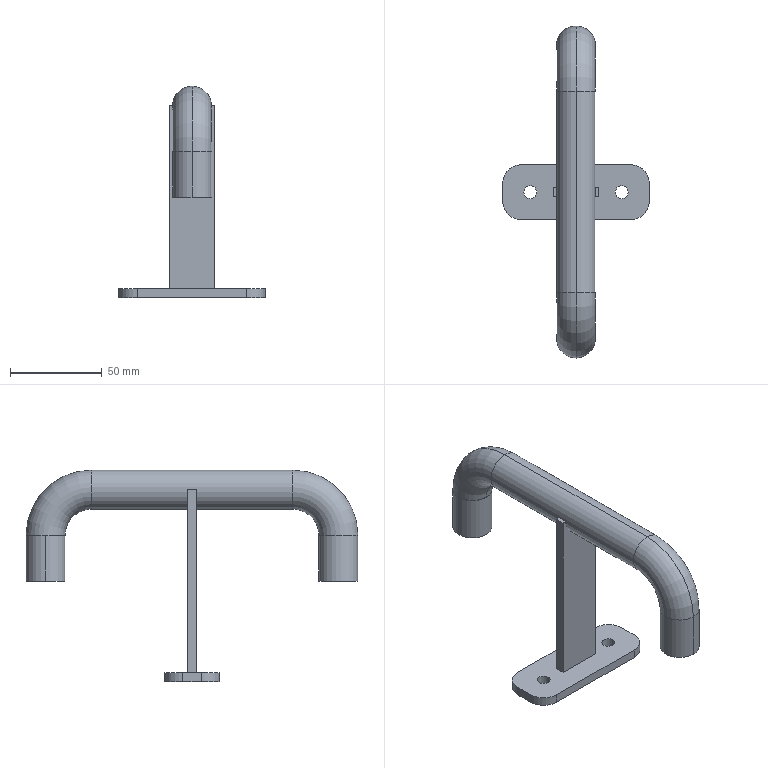Part | SolidWorks | features ICE 2, 3DProfileFeature 1, BossThin 1, Extrusion 1, Fillet 1, WeldMemberFeat 1, WeldmentFeature 1 | 7 solids | 56 faces | box 80 x 181.3 x 115.65 mm | volume 40270 mm3 | plane 27 | cylinder 21 | torus 8 | commonest cylinder face diameters 18.9 x6 21.3 x6 7 x4 20 x4 21 x1
STEP:
#1=CARTESIAN_POINT('',(61.5,-15.,5.));
#2=VERTEX_POINT('',#1);
#3=CARTESIAN_POINT('',(68.5,-15.,5.));
#4=VERTEX_POINT('',#3);
#5=CARTESIAN_POINT('',(65.,-15.,5.));
#6=DIRECTION('',(0.,0.,1.));
#7=DIRECTION('',(1.,0.,0.));
#8=AXIS2_PLACEMENT_3D('',#5,#6,#7);
#9=CIRCLE('',#8,3.5);
#10=EDGE_CURVE('',#2,#4,#9,.T.);
#11=ORIENTED_EDGE('',*,*,#10,.T.);
#12=CARTESIAN_POINT('',(68.5,-15.,0.));
#13=VERTEX_POINT('',#12);
#14=CARTESIAN_POINT('',(68.5,-15.,5.));
#15=DIRECTION('',(0.,0.,-1.));
#16=VECTOR('',#15,1000.);
#17=LINE('',#14,#16);
#18=EDGE_CURVE('',#4,#13,#17,.T.);
#19=ORIENTED_EDGE('',*,*,#18,.T.);
#20=CARTESIAN_POINT('',(61.5,-15.,0.));
#21=VERTEX_POINT('',#20);
#22=CARTESIAN_POINT('',(65.,-15.,0.));
#23=DIRECTION('',(0.,0.,1.));
#24=DIRECTION('',(1.,0.,0.));
#25=AXIS2_PLACEMENT_3D('',#22,#23,#24);
#26=CIRCLE('',#25,3.5);
#27=EDGE_CURVE('',#21,#13,#26,.T.);
#28=ORIENTED_EDGE('',*,*,#27,.F.);
#29=CARTESIAN_POINT('',(61.5,-15.,5.));
#30=DIRECTION('',(0.,0.,-1.));
#31=VECTOR('',#30,1000.);
#32=LINE('',#29,#31);
#33=EDGE_CURVE('',#2,#21,#32,.T.);
#34=ORIENTED_EDGE('',*,*,#33,.F.);
#35=EDGE_LOOP('',(#11,#19,#28,#34));
#36=FACE_OUTER_BOUND('',#35,.T.);
#37=CARTESIAN_POINT('',(65.,-15.,5.));
#38=DIRECTION('',(0.,0.,-1.));
#39=DIRECTION('',(-1.,0.,0.));
#40=AXIS2_PLACEMENT_3D('',#37,#38,#39);
#41=CYLINDRICAL_SURFACE('',#40,3.5);
#42=ADVANCED_FACE('',(#36),#41,.F.);
#43=CARTESIAN_POINT('',(11.5,-15.,5.));
#44=VERTEX_POINT('',#43);
#45=CARTESIAN_POINT('',(18.5,-15.,5.));
#46=VERTEX_POINT('',#45);
#47=CARTESIAN_POINT('',(15.,-15.,5.));
#48=DIRECTION('',(0.,0.,1.));
#49=DIRECTION('',(1.,0.,0.));
#50=AXIS2_PLACEMENT_3D('',#47,#48,#49);
#51=CIRCLE('',#50,3.5);
#52=EDGE_CURVE('',#44,#46,#51,.T.);
#53=ORIENTED_EDGE('',*,*,#52,.T.);
#54=CARTESIAN_POINT('',(18.5,-15.,0.));
#55=VERTEX_POINT('',#54);
#56=CARTESIAN_POINT('',(18.5,-15.,5.));
#57=DIRECTION('',(0.,0.,-1.));
#58=VECTOR('',#57,1000.);
#59=LINE('',#56,#58);
#60=EDGE_CURVE('',#46,#55,#59,.T.);
#61=ORIENTED_EDGE('',*,*,#60,.T.);
#62=CARTESIAN_POINT('',(11.5,-15.,0.));
#63=VERTEX_POINT('',#62);
#64=CARTESIAN_POINT('',(15.,-15.,0.));
#65=DIRECTION('',(0.,0.,1.));
#66=DIRECTION('',(1.,0.,0.));
#67=AXIS2_PLACEMENT_3D('',#64,#65,#66);
#68=CIRCLE('',#67,3.5);
#69=EDGE_CURVE('',#63,#55,#68,.T.);
#70=ORIENTED_EDGE('',*,*,#69,.F.);
#71=CARTESIAN_POINT('',(11.5,-15.,5.));
#72=DIRECTION('',(0.,0.,-1.));
#73=VECTOR('',#72,1000.);
#74=LINE('',#71,#73);
#75=EDGE_CURVE('',#44,#63,#74,.T.);
#76=ORIENTED_EDGE('',*,*,#75,.F.);
#77=EDGE_LOOP('',(#53,#61,#70,#76));
#78=FACE_OUTER_BOUND('',#77,.T.);
#79=CARTESIAN_POINT('',(15.,-15.,5.));
#80=DIRECTION('',(0.,0.,-1.));
#81=DIRECTION('',(-1.,0.,0.));
#82=AXIS2_PLACEMENT_3D('',#79,#80,#81);
#83=CYLINDRICAL_SURFACE('',#82,3.5);
#84=ADVANCED_FACE('',(#78),#83,.F.);
#85=ORIENTED_EDGE('',*,*,#52,.F.);
#86=CARTESIAN_POINT('',(15.,-15.,5.));
#87=DIRECTION('',(0.,0.,1.));
#88=DIRECTION('',(1.,0.,0.));
#89=AXIS2_PLACEMENT_3D('',#86,#87,#88);
#90=CIRCLE('',#89,3.5);
#91=EDGE_CURVE('',#46,#44,#90,.T.);
#92=ORIENTED_EDGE('',*,*,#91,.F.);
#93=EDGE_LOOP('',(#85,#92));
#94=FACE_BOUND('',#93,.T.);
#95=CARTESIAN_POINT('',(10.,-30.,5.));
#96=VERTEX_POINT('',#95);
#97=CARTESIAN_POINT('',(70.,-30.,5.));
#98=VERTEX_POINT('',#97);
#99=CARTESIAN_POINT('',(0.,-30.,5.));
#100=DIRECTION('',(1.,0.,0.));
#101=VECTOR('',#100,1000.);
#102=LINE('',#99,#101);
#103=EDGE_CURVE('',#96,#98,#102,.T.);
#104=ORIENTED_EDGE('',*,*,#103,.T.);
#105=CARTESIAN_POINT('',(80.,-20.,5.));
#106=VERTEX_POINT('',#105);
#107=CARTESIAN_POINT('',(70.,-20.,5.));
#108=DIRECTION('',(0.,0.,1.));
#109=DIRECTION('',(1.,0.,0.));
#110=AXIS2_PLACEMENT_3D('',#107,#108,#109);
#111=CIRCLE('',#110,10.);
#112=EDGE_CURVE('',#98,#106,#111,.T.);
#113=ORIENTED_EDGE('',*,*,#112,.T.);
#114=CARTESIAN_POINT('',(80.,-10.,5.));
#115=VERTEX_POINT('',#114);
#116=CARTESIAN_POINT('',(80.,0.,5.));
#117=DIRECTION('',(0.,1.,0.));
#118=VECTOR('',#117,1000.);
#119=LINE('',#116,#118);
#120=EDGE_CURVE('',#106,#115,#119,.T.);
#121=ORIENTED_EDGE('',*,*,#120,.T.);
#122=CARTESIAN_POINT('',(70.,0.,5.));
#123=VERTEX_POINT('',#122);
#124=CARTESIAN_POINT('',(70.,-10.,5.));
#125=DIRECTION('',(0.,0.,1.));
#126=DIRECTION('',(1.,0.,0.));
#127=AXIS2_PLACEMENT_3D('',#124,#125,#126);
#128=CIRCLE('',#127,10.);
#129=EDGE_CURVE('',#115,#123,#128,.T.);
#130=ORIENTED_EDGE('',*,*,#129,.T.);
#131=CARTESIAN_POINT('',(10.,0.,5.));
#132=VERTEX_POINT('',#131);
#133=CARTESIAN_POINT('',(0.,0.,5.));
#134=DIRECTION('',(-1.,0.,0.));
#135=VECTOR('',#134,1000.);
#136=LINE('',#133,#135);
#137=EDGE_CURVE('',#123,#132,#136,.T.);
#138=ORIENTED_EDGE('',*,*,#137,.T.);
#139=CARTESIAN_POINT('',(0.,-10.,5.));
#140=VERTEX_POINT('',#139);
#141=CARTESIAN_POINT('',(10.,-10.,5.));
#142=DIRECTION('',(0.,0.,1.));
#143=DIRECTION('',(1.,0.,0.));
#144=AXIS2_PLACEMENT_3D('',#141,#142,#143);
#145=CIRCLE('',#144,10.);
#146=EDGE_CURVE('',#132,#140,#145,.T.);
#147=ORIENTED_EDGE('',*,*,#146,.T.);
#148=CARTESIAN_POINT('',(0.,-20.,5.));
#149=VERTEX_POINT('',#148);
#150=CARTESIAN_POINT('',(0.,0.,5.));
#151=DIRECTION('',(0.,-1.,0.));
#152=VECTOR('',#151,1000.);
#153=LINE('',#150,#152);
#154=EDGE_CURVE('',#140,#149,#153,.T.);
#155=ORIENTED_EDGE('',*,*,#154,.T.);
#156=CARTESIAN_POINT('',(10.,-20.,5.));
#157=DIRECTION('',(0.,0.,1.));
#158=DIRECTION('',(1.,0.,0.));
#159=AXIS2_PLACEMENT_3D('',#156,#157,#158);
#160=CIRCLE('',#159,10.);
#161=EDGE_CURVE('',#149,#96,#160,.T.);
#162=ORIENTED_EDGE('',*,*,#161,.T.);
#163=EDGE_LOOP('',(#104,#113,#121,#130,#138,#147,#155,#162));
#164=FACE_OUTER_BOUND('',#163,.T.);
#165=ORIENTED_EDGE('',*,*,#10,.F.);
#166=CARTESIAN_POINT('',(65.,-15.,5.));
#167=DIRECTION('',(0.,0.,1.));
#168=DIRECTION('',(1.,0.,0.));
#169=AXIS2_PLACEMENT_3D('',#166,#167,#168);
#170=CIRCLE('',#169,3.5);
#171=EDGE_CURVE('',#4,#2,#170,.T.);
#172=ORIENTED_EDGE('',*,*,#171,.F.);
#173=EDGE_LOOP('',(#165,#172));
#174=FACE_BOUND('',#173,.T.);
#175=CARTESIAN_POINT('',(27.5,-17.5,5.));
#176=VERTEX_POINT('',#175);
#177=CARTESIAN_POINT('',(52.5,-17.5,5.));
#178=VERTEX_POINT('',#177);
#179=CARTESIAN_POINT('',(27.5,-17.5,5.));
#180=DIRECTION('',(1.,0.,0.));
#181=VECTOR('',#180,1000.);
#182=LINE('',#179,#181);
#183=EDGE_CURVE('',#176,#178,#182,.T.);
#184=ORIENTED_EDGE('',*,*,#183,.F.);
#185=CARTESIAN_POINT('',(27.5,-12.5,5.));
#186=VERTEX_POINT('',#185);
#187=CARTESIAN_POINT('',(27.5,-12.5,5.));
#188=DIRECTION('',(0.,-1.,0.));
#189=VECTOR('',#188,1000.);
#190=LINE('',#187,#189);
#191=EDGE_CURVE('',#186,#176,#190,.T.);
#192=ORIENTED_EDGE('',*,*,#191,.F.);
#193=CARTESIAN_POINT('',(52.5,-12.5,5.));
#194=VERTEX_POINT('',#193);
#195=CARTESIAN_POINT('',(27.5,-12.5,5.));
#196=DIRECTION('',(-1.,0.,0.));
#197=VECTOR('',#196,1000.);
#198=LINE('',#195,#197);
#199=EDGE_CURVE('',#194,#186,#198,.T.);
#200=ORIENTED_EDGE('',*,*,#199,.F.);
#201=CARTESIAN_POINT('',(52.5,-12.5,5.));
#202=DIRECTION('',(0.,1.,0.));
#203=VECTOR('',#202,1000.);
#204=LINE('',#201,#203);
#205=EDGE_CURVE('',#178,#194,#204,.T.);
#206=ORIENTED_EDGE('',*,*,#205,.F.);
#207=EDGE_LOOP('',(#184,#192,#200,#206));
#208=FACE_BOUND('',#207,.T.);
#209=CARTESIAN_POINT('',(0.,0.,5.));
#210=DIRECTION('',(0.,0.,1.));
#211=DIRECTION('',(1.,0.,0.));
#212=AXIS2_PLACEMENT_3D('',#209,#210,#211);
#213=PLANE('',#212);
#214=ADVANCED_FACE('',(#94,#164,#174,#208),#213,.T.);
#215=ORIENTED_EDGE('',*,*,#27,.T.);
#216=CARTESIAN_POINT('',(65.,-15.,0.));
#217=DIRECTION('',(0.,0.,1.));
#218=DIRECTION('',(1.,0.,0.));
#219=AXIS2_PLACEMENT_3D('',#216,#217,#218);
#220=CIRCLE('',#219,3.5);
#221=EDGE_CURVE('',#13,#21,#220,.T.);
#222=ORIENTED_EDGE('',*,*,#221,.T.);
#223=EDGE_LOOP('',(#215,#222));
#224=FACE_BOUND('',#223,.T.);
#225=ORIENTED_EDGE('',*,*,#69,.T.);
#226=CARTESIAN_POINT('',(15.,-15.,0.));
#227=DIRECTION('',(0.,0.,1.));
#228=DIRECTION('',(1.,0.,0.));
#229=AXIS2_PLACEMENT_3D('',#226,#227,#228);
#230=CIRCLE('',#229,3.5);
#231=EDGE_CURVE('',#55,#63,#230,.T.);
#232=ORIENTED_EDGE('',*,*,#231,.T.);
#233=EDGE_LOOP('',(#225,#232));
#234=FACE_BOUND('',#233,.T.);
#235=CARTESIAN_POINT('',(80.,-20.,0.));
#236=VERTEX_POINT('',#235);
#237=CARTESIAN_POINT('',(80.,-10.,0.));
#238=VERTEX_POINT('',#237);
#239=CARTESIAN_POINT('',(80.,0.,0.));
#240=DIRECTION('',(0.,1.,0.));
#241=VECTOR('',#240,1000.);
#242=LINE('',#239,#241);
#243=EDGE_CURVE('',#236,#238,#242,.T.);
#244=ORIENTED_EDGE('',*,*,#243,.F.);
#245=CARTESIAN_POINT('',(70.,-30.,0.));
#246=VERTEX_POINT('',#245);
#247=CARTESIAN_POINT('',(70.,-20.,0.));
#248=DIRECTION('',(0.,0.,-1.));
#249=DIRECTION('',(1.,0.,0.));
#250=AXIS2_PLACEMENT_3D('',#247,#248,#249);
#251=CIRCLE('',#250,10.);
#252=EDGE_CURVE('',#236,#246,#251,.T.);
#253=ORIENTED_EDGE('',*,*,#252,.T.);
#254=CARTESIAN_POINT('',(10.,-30.,0.));
#255=VERTEX_POINT('',#254);
#256=CARTESIAN_POINT('',(0.,-30.,0.));
#257=DIRECTION('',(1.,0.,0.));
#258=VECTOR('',#257,1000.);
#259=LINE('',#256,#258);
#260=EDGE_CURVE('',#255,#246,#259,.T.);
#261=ORIENTED_EDGE('',*,*,#260,.F.);
#262=CARTESIAN_POINT('',(0.,-20.,0.));
#263=VERTEX_POINT('',#262);
#264=CARTESIAN_POINT('',(10.,-20.,0.));
#265=DIRECTION('',(0.,0.,-1.));
#266=DIRECTION('',(1.,0.,0.));
#267=AXIS2_PLACEMENT_3D('',#264,#265,#266);
#268=CIRCLE('',#267,10.);
#269=EDGE_CURVE('',#255,#263,#268,.T.);
#270=ORIENTED_EDGE('',*,*,#269,.T.);
#271=CARTESIAN_POINT('',(0.,-10.,0.));
#272=VERTEX_POINT('',#271);
#273=CARTESIAN_POINT('',(0.,0.,0.));
#274=DIRECTION('',(0.,-1.,0.));
#275=VECTOR('',#274,1000.);
#276=LINE('',#273,#275);
#277=EDGE_CURVE('',#272,#263,#276,.T.);
#278=ORIENTED_EDGE('',*,*,#277,.F.);
#279=CARTESIAN_POINT('',(10.,0.,0.));
#280=VERTEX_POINT('',#279);
#281=CARTESIAN_POINT('',(10.,-10.,0.));
#282=DIRECTION('',(0.,0.,-1.));
#283=DIRECTION('',(1.,0.,0.));
#284=AXIS2_PLACEMENT_3D('',#281,#282,#283);
#285=CIRCLE('',#284,10.);
#286=EDGE_CURVE('',#272,#280,#285,.T.);
#287=ORIENTED_EDGE('',*,*,#286,.T.);
#288=CARTESIAN_POINT('',(70.,0.,0.));
#289=VERTEX_POINT('',#288);
#290=CARTESIAN_POINT('',(0.,0.,0.));
#291=DIRECTION('',(-1.,0.,0.));
#292=VECTOR('',#291,1000.);
#293=LINE('',#290,#292);
#294=EDGE_CURVE('',#289,#280,#293,.T.);
#295=ORIENTED_EDGE('',*,*,#294,.F.);
#296=CARTESIAN_POINT('',(70.,-10.,0.));
#297=DIRECTION('',(0.,0.,-1.));
#298=DIRECTION('',(1.,0.,0.));
#299=AXIS2_PLACEMENT_3D('',#296,#297,#298);
#300=CIRCLE('',#299,10.);
#301=EDGE_CURVE('',#289,#238,#300,.T.);
#302=ORIENTED_EDGE('',*,*,#301,.T.);
#303=EDGE_LOOP('',(#244,#253,#261,#270,#278,#287,#295,#302));
#304=FACE_OUTER_BOUND('',#303,.T.);
#305=CARTESIAN_POINT('',(27.5,-12.5,0.));
#306=VERTEX_POINT('',#305);
#307=CARTESIAN_POINT('',(27.5,-17.5,0.));
#308=VERTEX_POINT('',#307);
#309=CARTESIAN_POINT('',(27.5,-12.5,0.));
#310=DIRECTION('',(0.,-1.,0.));
#311=VECTOR('',#310,1000.);
#312=LINE('',#309,#311);
#313=EDGE_CURVE('',#306,#308,#312,.T.);
#314=ORIENTED_EDGE('',*,*,#313,.T.);
#315=CARTESIAN_POINT('',(52.5,-17.5,0.));
#316=VERTEX_POINT('',#315);
#317=CARTESIAN_POINT('',(27.5,-17.5,0.));
#318=DIRECTION('',(1.,0.,0.));
#319=VECTOR('',#318,1000.);
#320=LINE('',#317,#319);
#321=EDGE_CURVE('',#308,#316,#320,.T.);
#322=ORIENTED_EDGE('',*,*,#321,.T.);
#323=CARTESIAN_POINT('',(52.5,-12.5,0.));
#324=VERTEX_POINT('',#323);
#325=CARTESIAN_POINT('',(52.5,-12.5,0.));
#326=DIRECTION('',(0.,1.,0.));
#327=VECTOR('',#326,1000.);
#328=LINE('',#325,#327);
#329=EDGE_CURVE('',#316,#324,#328,.T.);
#330=ORIENTED_EDGE('',*,*,#329,.T.);
#331=CARTESIAN_POINT('',(27.5,-12.5,0.));
#332=DIRECTION('',(-1.,0.,0.));
#333=VECTOR('',#332,1000.);
#334=LINE('',#331,#333);
#335=EDGE_CURVE('',#324,#306,#334,.T.);
#336=ORIENTED_EDGE('',*,*,#335,.T.);
#337=EDGE_LOOP('',(#314,#322,#330,#336));
#338=FACE_BOUND('',#337,.T.);
#339=CARTESIAN_POINT('',(0.,0.,0.));
#340=DIRECTION('',(0.,0.,1.));
#341=DIRECTION('',(1.,0.,0.));
#342=AXIS2_PLACEMENT_3D('',#339,#340,#341);
#343=PLANE('',#342);
#344=ADVANCED_FACE('',(#224,#234,#304,#338),#343,.F.);
#345=ORIENTED_EDGE('',*,*,#154,.F.);
#346=CARTESIAN_POINT('',(0.,-10.,5.));
#347=DIRECTION('',(0.,0.,-1.));
#348=VECTOR('',#347,1000.);
#349=LINE('',#346,#348);
#350=EDGE_CURVE('',#140,#272,#349,.T.);
#351=ORIENTED_EDGE('',*,*,#350,.T.);
#352=ORIENTED_EDGE('',*,*,#277,.T.);
#353=CARTESIAN_POINT('',(0.,-20.,5.));
#354=DIRECTION('',(0.,0.,1.));
#355=VECTOR('',#354,1000.);
#356=LINE('',#353,#355);
#357=EDGE_CURVE('',#263,#149,#356,.T.);
#358=ORIENTED_EDGE('',*,*,#357,.T.);
#359=EDGE_LOOP('',(#345,#351,#352,#358));
#360=FACE_OUTER_BOUND('',#359,.T.);
#361=CARTESIAN_POINT('',(0.,0.,5.));
#362=DIRECTION('',(1.,0.,0.));
#363=DIRECTION('',(0.,0.,-1.));
#364=AXIS2_PLACEMENT_3D('',#361,#362,#363);
#365=PLANE('',#364);
#366=ADVANCED_FACE('',(#360),#365,.F.);
#367=ORIENTED_EDGE('',*,*,#260,.T.);
#368=CARTESIAN_POINT('',(70.,-30.,5.));
#369=DIRECTION('',(0.,0.,1.));
#370=VECTOR('',#369,1000.);
#371=LINE('',#368,#370);
#372=EDGE_CURVE('',#246,#98,#371,.T.);
#373=ORIENTED_EDGE('',*,*,#372,.T.);
#374=ORIENTED_EDGE('',*,*,#103,.F.);
#375=CARTESIAN_POINT('',(10.,-30.,5.));
#376=DIRECTION('',(0.,0.,-1.));
#377=VECTOR('',#376,1000.);
#378=LINE('',#375,#377);
#379=EDGE_CURVE('',#96,#255,#378,.T.);
#380=ORIENTED_EDGE('',*,*,#379,.T.);
#381=EDGE_LOOP('',(#367,#373,#374,#380));
#382=FACE_OUTER_BOUND('',#381,.T.);
#383=CARTESIAN_POINT('',(0.,-30.,5.));
#384=DIRECTION('',(0.,1.,0.));
#385=DIRECTION('',(0.,0.,1.));
#386=AXIS2_PLACEMENT_3D('',#383,#384,#385);
#387=PLANE('',#386);
#388=ADVANCED_FACE('',(#382),#387,.F.);
#389=ORIENTED_EDGE('',*,*,#120,.F.);
#390=CARTESIAN_POINT('',(80.,-20.,5.));
#391=DIRECTION('',(0.,0.,-1.));
#392=VECTOR('',#391,1000.);
#393=LINE('',#390,#392);
#394=EDGE_CURVE('',#106,#236,#393,.T.);
#395=ORIENTED_EDGE('',*,*,#394,.T.);
#396=ORIENTED_EDGE('',*,*,#243,.T.);
#397=CARTESIAN_POINT('',(80.,-10.,5.));
#398=DIRECTION('',(0.,0.,1.));
#399=VECTOR('',#398,1000.);
#400=LINE('',#397,#399);
#401=EDGE_CURVE('',#238,#115,#400,.T.);
#402=ORIENTED_EDGE('',*,*,#401,.T.);
#403=EDGE_LOOP('',(#389,#395,#396,#402));
#404=FACE_OUTER_BOUND('',#403,.T.);
#405=CARTESIAN_POINT('',(80.,0.,5.));
#406=DIRECTION('',(-1.,0.,0.));
#407=DIRECTION('',(0.,0.,1.));
#408=AXIS2_PLACEMENT_3D('',#405,#406,#407);
#409=PLANE('',#408);
#410=ADVANCED_FACE('',(#404),#409,.F.);
#411=ORIENTED_EDGE('',*,*,#137,.F.);
#412=CARTESIAN_POINT('',(70.,0.,5.));
#413=DIRECTION('',(0.,0.,-1.));
#414=VECTOR('',#413,1000.);
#415=LINE('',#412,#414);
#416=EDGE_CURVE('',#123,#289,#415,.T.);
#417=ORIENTED_EDGE('',*,*,#416,.T.);
#418=ORIENTED_EDGE('',*,*,#294,.T.);
#419=CARTESIAN_POINT('',(10.,0.,5.));
#420=DIRECTION('',(0.,0.,1.));
#421=VECTOR('',#420,1000.);
#422=LINE('',#419,#421);
#423=EDGE_CURVE('',#280,#132,#422,.T.);
#424=ORIENTED_EDGE('',*,*,#423,.T.);
#425=EDGE_LOOP('',(#411,#417,#418,#424));
#426=FACE_OUTER_BOUND('',#425,.T.);
#427=CARTESIAN_POINT('',(0.,0.,5.));
#428=DIRECTION('',(0.,-1.,0.));
#429=DIRECTION('',(0.,0.,-1.));
#430=AXIS2_PLACEMENT_3D('',#427,#428,#429);
#431=PLANE('',#430);
#432=ADVANCED_FACE('',(#426),#431,.F.);
#433=ORIENTED_EDGE('',*,*,#60,.F.);
#434=ORIENTED_EDGE('',*,*,#91,.T.);
#435=ORIENTED_EDGE('',*,*,#75,.T.);
#436=ORIENTED_EDGE('',*,*,#231,.F.);
#437=EDGE_LOOP('',(#433,#434,#435,#436));
#438=FACE_OUTER_BOUND('',#437,.T.);
#439=CARTESIAN_POINT('',(15.,-15.,5.));
#440=DIRECTION('',(0.,0.,-1.));
#441=DIRECTION('',(-1.,0.,0.));
#442=AXIS2_PLACEMENT_3D('',#439,#440,#441);
#443=CYLINDRICAL_SURFACE('',#442,3.5);
#444=ADVANCED_FACE('',(#438),#443,.F.);
#445=ORIENTED_EDGE('',*,*,#18,.F.);
#446=ORIENTED_EDGE('',*,*,#171,.T.);
#447=ORIENTED_EDGE('',*,*,#33,.T.);
#448=ORIENTED_EDGE('',*,*,#221,.F.);
#449=EDGE_LOOP('',(#445,#446,#447,#448));
#450=FACE_OUTER_BOUND('',#449,.T.);
#451=CARTESIAN_POINT('',(65.,-15.,5.));
#452=DIRECTION('',(0.,0.,-1.));
#453=DIRECTION('',(-1.,0.,0.));
#454=AXIS2_PLACEMENT_3D('',#451,#452,#453);
#455=CYLINDRICAL_SURFACE('',#454,3.5);
#456=ADVANCED_FACE('',(#450),#455,.F.);
#457=ORIENTED_EDGE('',*,*,#313,.F.);
#458=CARTESIAN_POINT('',(27.5,-12.5,5.));
#459=DIRECTION('',(0.,0.,-1.));
#460=VECTOR('',#459,1000.);
#461=LINE('',#458,#460);
#462=EDGE_CURVE('',#186,#306,#461,.T.);
#463=ORIENTED_EDGE('',*,*,#462,.F.);
#464=ORIENTED_EDGE('',*,*,#191,.T.);
#465=CARTESIAN_POINT('',(27.5,-17.5,5.));
#466=DIRECTION('',(0.,0.,-1.));
#467=VECTOR('',#466,1000.);
#468=LINE('',#465,#467);
#469=EDGE_CURVE('',#176,#308,#468,.T.);
#470=ORIENTED_EDGE('',*,*,#469,.T.);
#471=EDGE_LOOP('',(#457,#463,#464,#470));
#472=FACE_OUTER_BOUND('',#471,.T.);
#473=CARTESIAN_POINT('',(27.5,-12.5,5.));
#474=DIRECTION('',(1.,0.,0.));
#475=DIRECTION('',(0.,0.,-1.));
#476=AXIS2_PLACEMENT_3D('',#473,#474,#475);
#477=PLANE('',#476);
#478=ADVANCED_FACE('',(#472),#477,.T.);
#479=ORIENTED_EDGE('',*,*,#321,.F.);
#480=ORIENTED_EDGE('',*,*,#469,.F.);
#481=ORIENTED_EDGE('',*,*,#183,.T.);
#482=CARTESIAN_POINT('',(52.5,-17.5,5.));
#483=DIRECTION('',(0.,0.,-1.));
#484=VECTOR('',#483,1000.);
#485=LINE('',#482,#484);
#486=EDGE_CURVE('',#178,#316,#485,.T.);
#487=ORIENTED_EDGE('',*,*,#486,.T.);
#488=EDGE_LOOP('',(#479,#480,#481,#487));
#489=FACE_OUTER_BOUND('',#488,.T.);
#490=CARTESIAN_POINT('',(27.5,-17.5,5.));
#491=DIRECTION('',(0.,1.,0.));
#492=DIRECTION('',(-1.,0.,0.));
#493=AXIS2_PLACEMENT_3D('',#490,#491,#492);
#494=PLANE('',#493);
#495=ADVANCED_FACE('',(#489),#494,.T.);
#496=ORIENTED_EDGE('',*,*,#329,.F.);
#497=ORIENTED_EDGE('',*,*,#486,.F.);
#498=ORIENTED_EDGE('',*,*,#205,.T.);
#499=CARTESIAN_POINT('',(52.5,-12.5,5.));
#500=DIRECTION('',(0.,0.,-1.));
#501=VECTOR('',#500,1000.);
#502=LINE('',#499,#501);
#503=EDGE_CURVE('',#194,#324,#502,.T.);
#504=ORIENTED_EDGE('',*,*,#503,.T.);
#505=EDGE_LOOP('',(#496,#497,#498,#504));
#506=FACE_OUTER_BOUND('',#505,.T.);
#507=CARTESIAN_POINT('',(52.5,-12.5,5.));
#508=DIRECTION('',(-1.,0.,0.));
#509=DIRECTION('',(0.,0.,1.));
#510=AXIS2_PLACEMENT_3D('',#507,#508,#509);
#511=PLANE('',#510);
#512=ADVANCED_FACE('',(#506),#511,.T.);
#513=ORIENTED_EDGE('',*,*,#335,.F.);
#514=ORIENTED_EDGE('',*,*,#503,.F.);
#515=ORIENTED_EDGE('',*,*,#199,.T.);
#516=ORIENTED_EDGE('',*,*,#462,.T.);
#517=EDGE_LOOP('',(#513,#514,#515,#516));
#518=FACE_OUTER_BOUND('',#517,.T.);
#519=CARTESIAN_POINT('',(27.5,-12.5,5.));
#520=DIRECTION('',(0.,-1.,0.));
#521=DIRECTION('',(0.,0.,-1.));
#522=AXIS2_PLACEMENT_3D('',#519,#520,#521);
#523=PLANE('',#522);
#524=ADVANCED_FACE('',(#518),#523,.T.);
#525=ORIENTED_EDGE('',*,*,#112,.F.);
#526=ORIENTED_EDGE('',*,*,#372,.F.);
#527=ORIENTED_EDGE('',*,*,#252,.F.);
#528=ORIENTED_EDGE('',*,*,#394,.F.);
#529=EDGE_LOOP('',(#525,#526,#527,#528));
#530=FACE_OUTER_BOUND('',#529,.T.);
#531=CARTESIAN_POINT('',(70.,-20.,5.));
#532=DIRECTION('',(0.,0.,-1.));
#533=DIRECTION('',(-1.,0.,0.));
#534=AXIS2_PLACEMENT_3D('',#531,#532,#533);
#535=CYLINDRICAL_SURFACE('',#534,10.);
#536=ADVANCED_FACE('',(#530),#535,.T.);
#537=ORIENTED_EDGE('',*,*,#129,.F.);
#538=ORIENTED_EDGE('',*,*,#401,.F.);
#539=ORIENTED_EDGE('',*,*,#301,.F.);
#540=ORIENTED_EDGE('',*,*,#416,.F.);
#541=EDGE_LOOP('',(#537,#538,#539,#540));
#542=FACE_OUTER_BOUND('',#541,.T.);
#543=CARTESIAN_POINT('',(70.,-10.,5.));
#544=DIRECTION('',(0.,0.,-1.));
#545=DIRECTION('',(-1.,0.,0.));
#546=AXIS2_PLACEMENT_3D('',#543,#544,#545);
#547=CYLINDRICAL_SURFACE('',#546,10.);
#548=ADVANCED_FACE('',(#542),#547,.T.);
#549=ORIENTED_EDGE('',*,*,#146,.F.);
#550=ORIENTED_EDGE('',*,*,#423,.F.);
#551=ORIENTED_EDGE('',*,*,#286,.F.);
#552=ORIENTED_EDGE('',*,*,#350,.F.);
#553=EDGE_LOOP('',(#549,#550,#551,#552));
#554=FACE_OUTER_BOUND('',#553,.T.);
#555=CARTESIAN_POINT('',(10.,-10.,5.));
#556=DIRECTION('',(0.,0.,-1.));
#557=DIRECTION('',(-1.,0.,0.));
#558=AXIS2_PLACEMENT_3D('',#555,#556,#557);
#559=CYLINDRICAL_SURFACE('',#558,10.);
#560=ADVANCED_FACE('',(#554),#559,.T.);
#561=ORIENTED_EDGE('',*,*,#161,.F.);
#562=ORIENTED_EDGE('',*,*,#357,.F.);
#563=ORIENTED_EDGE('',*,*,#269,.F.);
#564=ORIENTED_EDGE('',*,*,#379,.F.);
#565=EDGE_LOOP('',(#561,#562,#563,#564));
#566=FACE_OUTER_BOUND('',#565,.T.);
#567=CARTESIAN_POINT('',(10.,-20.,5.));
#568=DIRECTION('',(0.,0.,-1.));
#569=DIRECTION('',(-1.,0.,0.));
#570=AXIS2_PLACEMENT_3D('',#567,#568,#569);
#571=CYLINDRICAL_SURFACE('',#570,10.);
#572=ADVANCED_FACE('',(#566),#571,.T.);
#573=CLOSED_SHELL('',(#42,#84,#214,#344,#366,#388,#410,#432,#444,#456,#478,#495,#512,#524,#536,#548,#560,#572));
#574=MANIFOLD_SOLID_BREP('',#573);
#575=CARTESIAN_POINT('',(29.5,-12.5,105.));
#576=VERTEX_POINT('',#575);
#577=CARTESIAN_POINT('',(29.5,-17.5,105.));
#578=VERTEX_POINT('',#577);
#579=CARTESIAN_POINT('',(29.5,0.,105.));
#580=DIRECTION('',(0.,-1.,0.));
#581=VECTOR('',#580,1000.);
#582=LINE('',#579,#581);
#583=EDGE_CURVE('',#576,#578,#582,.T.);
#584=ORIENTED_EDGE('',*,*,#583,.F.);
#585=CARTESIAN_POINT('',(27.5,-12.5,105.));
#586=VERTEX_POINT('',#585);
#587=CARTESIAN_POINT('',(52.5,-12.5,105.));
#588=DIRECTION('',(-1.,0.,0.));
#589=VECTOR('',#588,1000.);
#590=LINE('',#587,#589);
#591=EDGE_CURVE('',#576,#586,#590,.T.);
#592=ORIENTED_EDGE('',*,*,#591,.T.);
#593=CARTESIAN_POINT('',(27.5,-17.5,105.));
#594=VERTEX_POINT('',#593);
#595=CARTESIAN_POINT('',(27.5,-12.5,105.));
#596=DIRECTION('',(0.,-1.,0.));
#597=VECTOR('',#596,1000.);
#598=LINE('',#595,#597);
#599=EDGE_CURVE('',#586,#594,#598,.T.);
#600=ORIENTED_EDGE('',*,*,#599,.T.);
#601=CARTESIAN_POINT('',(27.5,-17.5,105.));
#602=DIRECTION('',(1.,0.,0.));
#603=VECTOR('',#602,1000.);
#604=LINE('',#601,#603);
#605=EDGE_CURVE('',#594,#578,#604,.T.);
#606=ORIENTED_EDGE('',*,*,#605,.T.);
#607=EDGE_LOOP('',(#584,#592,#600,#606));
#608=FACE_OUTER_BOUND('',#607,.T.);
#609=CARTESIAN_POINT('',(0.,0.,105.));
#610=DIRECTION('',(0.,0.,1.));
#611=DIRECTION('',(1.,0.,0.));
#612=AXIS2_PLACEMENT_3D('',#609,#610,#611);
#613=PLANE('',#612);
#614=ADVANCED_FACE('',(#608),#613,.T.);
#615=CARTESIAN_POINT('',(50.5,-17.5,105.));
#616=VERTEX_POINT('',#615);
#617=CARTESIAN_POINT('',(52.5,-17.5,105.));
#618=VERTEX_POINT('',#617);
#619=CARTESIAN_POINT('',(27.5,-17.5,105.));
#620=DIRECTION('',(1.,0.,0.));
#621=VECTOR('',#620,1000.);
#622=LINE('',#619,#621);
#623=EDGE_CURVE('',#616,#618,#622,.T.);
#624=ORIENTED_EDGE('',*,*,#623,.F.);
#625=CARTESIAN_POINT('',(40.,-17.5,105.));
#626=DIRECTION('',(0.,-1.,0.));
#627=DIRECTION('',(1.,0.,0.));
#628=AXIS2_PLACEMENT_3D('',#625,#626,#627);
#629=CIRCLE('',#628,10.5);
#630=EDGE_CURVE('',#578,#616,#629,.T.);
#631=ORIENTED_EDGE('',*,*,#630,.F.);
#632=ORIENTED_EDGE('',*,*,#605,.F.);
#633=CARTESIAN_POINT('',(27.5,-17.5,5.));
#634=VERTEX_POINT('',#633);
#635=CARTESIAN_POINT('',(27.5,-17.5,105.));
#636=DIRECTION('',(0.,0.,-1.));
#637=VECTOR('',#636,1000.);
#638=LINE('',#635,#637);
#639=EDGE_CURVE('',#594,#634,#638,.T.);
#640=ORIENTED_EDGE('',*,*,#639,.T.);
#641=CARTESIAN_POINT('',(52.5,-17.5,5.));
#642=VERTEX_POINT('',#641);
#643=CARTESIAN_POINT('',(27.5,-17.5,5.));
#644=DIRECTION('',(1.,0.,0.));
#645=VECTOR('',#644,1000.);
#646=LINE('',#643,#645);
#647=EDGE_CURVE('',#634,#642,#646,.T.);
#648=ORIENTED_EDGE('',*,*,#647,.T.);
#649=CARTESIAN_POINT('',(52.5,-17.5,105.));
#650=DIRECTION('',(0.,0.,-1.));
#651=VECTOR('',#650,1000.);
#652=LINE('',#649,#651);
#653=EDGE_CURVE('',#618,#642,#652,.T.);
#654=ORIENTED_EDGE('',*,*,#653,.F.);
#655=EDGE_LOOP('',(#624,#631,#632,#640,#648,#654));
#656=FACE_OUTER_BOUND('',#655,.T.);
#657=CARTESIAN_POINT('',(27.5,-17.5,105.));
#658=DIRECTION('',(0.,1.,0.));
#659=DIRECTION('',(-1.,0.,0.));
#660=AXIS2_PLACEMENT_3D('',#657,#658,#659);
#661=PLANE('',#660);
#662=ADVANCED_FACE('',(#656),#661,.F.);
#663=CARTESIAN_POINT('',(52.5,-12.5,5.));
#664=VERTEX_POINT('',#663);
#665=CARTESIAN_POINT('',(52.5,-17.5,5.));
#666=DIRECTION('',(0.,1.,0.));
#667=VECTOR('',#666,1000.);
#668=LINE('',#665,#667);
#669=EDGE_CURVE('',#642,#664,#668,.T.);
#670=ORIENTED_EDGE('',*,*,#669,.T.);
#671=CARTESIAN_POINT('',(52.5,-12.5,105.));
#672=VERTEX_POINT('',#671);
#673=CARTESIAN_POINT('',(52.5,-12.5,105.));
#674=DIRECTION('',(0.,0.,-1.));
#675=VECTOR('',#674,1000.);
#676=LINE('',#673,#675);
#677=EDGE_CURVE('',#672,#664,#676,.T.);
#678=ORIENTED_EDGE('',*,*,#677,.F.);
#679=CARTESIAN_POINT('',(52.5,-17.5,105.));
#680=DIRECTION('',(0.,1.,0.));
#681=VECTOR('',#680,1000.);
#682=LINE('',#679,#681);
#683=EDGE_CURVE('',#618,#672,#682,.T.);
#684=ORIENTED_EDGE('',*,*,#683,.F.);
#685=ORIENTED_EDGE('',*,*,#653,.T.);
#686=EDGE_LOOP('',(#670,#678,#684,#685));
#687=FACE_OUTER_BOUND('',#686,.T.);
#688=CARTESIAN_POINT('',(52.5,-17.5,105.));
#689=DIRECTION('',(-1.,0.,0.));
#690=DIRECTION('',(0.,0.,1.));
#691=AXIS2_PLACEMENT_3D('',#688,#689,#690);
#692=PLANE('',#691);
#693=ADVANCED_FACE('',(#687),#692,.F.);
#694=ORIENTED_EDGE('',*,*,#591,.F.);
#695=CARTESIAN_POINT('',(50.5,-12.5,105.));
#696=VERTEX_POINT('',#695);
#697=CARTESIAN_POINT('',(40.,-12.5,105.));
#698=DIRECTION('',(0.,-1.,0.));
#699=DIRECTION('',(0.,0.,-1.));
#700=AXIS2_PLACEMENT_3D('',#697,#698,#699);
#701=CIRCLE('',#700,10.5);
#702=EDGE_CURVE('',#576,#696,#701,.T.);
#703=ORIENTED_EDGE('',*,*,#702,.T.);
#704=CARTESIAN_POINT('',(52.5,-12.5,105.));
#705=DIRECTION('',(-1.,0.,0.));
#706=VECTOR('',#705,1000.);
#707=LINE('',#704,#706);
#708=EDGE_CURVE('',#672,#696,#707,.T.);
#709=ORIENTED_EDGE('',*,*,#708,.F.);
#710=ORIENTED_EDGE('',*,*,#677,.T.);
#711=CARTESIAN_POINT('',(27.5,-12.5,5.));
#712=VERTEX_POINT('',#711);
#713=CARTESIAN_POINT('',(52.5,-12.5,5.));
#714=DIRECTION('',(-1.,0.,0.));
#715=VECTOR('',#714,1000.);
#716=LINE('',#713,#715);
#717=EDGE_CURVE('',#664,#712,#716,.T.);
#718=ORIENTED_EDGE('',*,*,#717,.T.);
#719=CARTESIAN_POINT('',(27.5,-12.5,105.));
#720=DIRECTION('',(0.,0.,-1.));
#721=VECTOR('',#720,1000.);
#722=LINE('',#719,#721);
#723=EDGE_CURVE('',#586,#712,#722,.T.);
#724=ORIENTED_EDGE('',*,*,#723,.F.);
#725=EDGE_LOOP('',(#694,#703,#709,#710,#718,#724));
#726=FACE_OUTER_BOUND('',#725,.T.);
#727=CARTESIAN_POINT('',(52.5,-12.5,105.));
#728=DIRECTION('',(0.,-1.,0.));
#729=DIRECTION('',(0.,0.,-1.));
#730=AXIS2_PLACEMENT_3D('',#727,#728,#729);
#731=PLANE('',#730);
#732=ADVANCED_FACE('',(#726),#731,.F.);
#733=CARTESIAN_POINT('',(27.5,-12.5,5.));
#734=DIRECTION('',(0.,-1.,0.));
#735=VECTOR('',#734,1000.);
#736=LINE('',#733,#735);
#737=EDGE_CURVE('',#712,#634,#736,.T.);
#738=ORIENTED_EDGE('',*,*,#737,.T.);
#739=ORIENTED_EDGE('',*,*,#639,.F.);
#740=ORIENTED_EDGE('',*,*,#599,.F.);
#741=ORIENTED_EDGE('',*,*,#723,.T.);
#742=EDGE_LOOP('',(#738,#739,#740,#741));
#743=FACE_OUTER_BOUND('',#742,.T.);
#744=CARTESIAN_POINT('',(27.5,-12.5,105.));
#745=DIRECTION('',(1.,0.,0.));
#746=DIRECTION('',(0.,0.,-1.));
#747=AXIS2_PLACEMENT_3D('',#744,#745,#746);
#748=PLANE('',#747);
#749=ADVANCED_FACE('',(#743),#748,.F.);
#750=CARTESIAN_POINT('',(50.5,0.,105.));
#751=DIRECTION('',(0.,1.,0.));
#752=VECTOR('',#751,1000.);
#753=LINE('',#750,#752);
#754=EDGE_CURVE('',#616,#696,#753,.T.);
#755=ORIENTED_EDGE('',*,*,#754,.F.);
#756=ORIENTED_EDGE('',*,*,#623,.T.);
#757=ORIENTED_EDGE('',*,*,#683,.T.);
#758=ORIENTED_EDGE('',*,*,#708,.T.);
#759=EDGE_LOOP('',(#755,#756,#757,#758));
#760=FACE_OUTER_BOUND('',#759,.T.);
#761=CARTESIAN_POINT('',(0.,0.,105.));
#762=DIRECTION('',(0.,0.,1.));
#763=DIRECTION('',(1.,0.,0.));
#764=AXIS2_PLACEMENT_3D('',#761,#762,#763);
#765=PLANE('',#764);
#766=ADVANCED_FACE('',(#760),#765,.T.);
#767=ORIENTED_EDGE('',*,*,#647,.F.);
#768=ORIENTED_EDGE('',*,*,#737,.F.);
#769=ORIENTED_EDGE('',*,*,#717,.F.);
#770=ORIENTED_EDGE('',*,*,#669,.F.);
#771=EDGE_LOOP('',(#767,#768,#769,#770));
#772=FACE_OUTER_BOUND('',#771,.T.);
#773=CARTESIAN_POINT('',(0.,0.,5.));
#774=DIRECTION('',(0.,0.,1.));
#775=DIRECTION('',(1.,0.,0.));
#776=AXIS2_PLACEMENT_3D('',#773,#774,#775);
#777=PLANE('',#776);
#778=ADVANCED_FACE('',(#772),#777,.F.);
#779=ORIENTED_EDGE('',*,*,#583,.T.);
#780=ORIENTED_EDGE('',*,*,#630,.T.);
#781=ORIENTED_EDGE('',*,*,#754,.T.);
#782=ORIENTED_EDGE('',*,*,#702,.F.);
#783=EDGE_LOOP('',(#779,#780,#781,#782));
#784=FACE_OUTER_BOUND('',#783,.T.);
#785=CARTESIAN_POINT('',(40.,0.,105.));
#786=DIRECTION('',(0.,-1.,0.));
#787=DIRECTION('',(1.,0.,0.));
#788=AXIS2_PLACEMENT_3D('',#785,#786,#787);
#789=CYLINDRICAL_SURFACE('',#788,10.5);
#790=ADVANCED_FACE('',(#784),#789,.F.);
#791=CLOSED_SHELL('',(#614,#662,#693,#732,#749,#766,#778,#790));
#792=MANIFOLD_SOLID_BREP('',#791);
#793=CARTESIAN_POINT('',(40.,-70.,94.35));
#794=VERTEX_POINT('',#793);
#795=CARTESIAN_POINT('',(40.,-70.,115.65));
#796=VERTEX_POINT('',#795);
#797=CARTESIAN_POINT('',(40.,-70.,105.));
#798=DIRECTION('',(0.,-1.,0.));
#799=DIRECTION('',(0.,0.,-1.));
#800=AXIS2_PLACEMENT_3D('',#797,#798,#799);
#801=CIRCLE('',#800,10.65);
#802=EDGE_CURVE('',#794,#796,#801,.T.);
#803=ORIENTED_EDGE('',*,*,#802,.F.);
#804=CARTESIAN_POINT('',(40.,40.,94.35));
#805=VERTEX_POINT('',#804);
#806=CARTESIAN_POINT('',(40.,-70.,94.35));
#807=DIRECTION('',(0.,1.,0.));
#808=VECTOR('',#807,1000.);
#809=LINE('',#806,#808);
#810=EDGE_CURVE('',#794,#805,#809,.T.);
#811=ORIENTED_EDGE('',*,*,#810,.T.);
#812=CARTESIAN_POINT('',(40.,40.,115.65));
#813=VERTEX_POINT('',#812);
#814=CARTESIAN_POINT('',(40.,40.,105.));
#815=DIRECTION('',(0.,1.,0.));
#816=DIRECTION('',(0.,0.,1.));
#817=AXIS2_PLACEMENT_3D('',#814,#815,#816);
#818=CIRCLE('',#817,10.65);
#819=EDGE_CURVE('',#813,#805,#818,.T.);
#820=ORIENTED_EDGE('',*,*,#819,.F.);
#821=CARTESIAN_POINT('',(40.,-70.,115.65));
#822=DIRECTION('',(0.,1.,0.));
#823=VECTOR('',#822,1000.);
#824=LINE('',#821,#823);
#825=EDGE_CURVE('',#796,#813,#824,.T.);
#826=ORIENTED_EDGE('',*,*,#825,.F.);
#827=EDGE_LOOP('',(#803,#811,#820,#826));
#828=FACE_OUTER_BOUND('',#827,.T.);
#829=CARTESIAN_POINT('',(40.,-70.,105.));
#830=DIRECTION('',(0.,1.,0.));
#831=DIRECTION('',(0.,0.,1.));
#832=AXIS2_PLACEMENT_3D('',#829,#830,#831);
#833=CYLINDRICAL_SURFACE('',#832,10.65);
#834=ADVANCED_FACE('',(#828),#833,.T.);
#835=CARTESIAN_POINT('',(40.,-70.,114.45));
#836=VERTEX_POINT('',#835);
#837=CARTESIAN_POINT('',(40.,-70.,95.55));
#838=VERTEX_POINT('',#837);
#839=CARTESIAN_POINT('',(40.,-70.,105.));
#840=DIRECTION('',(0.,-1.,0.));
#841=DIRECTION('',(0.,0.,-1.));
#842=AXIS2_PLACEMENT_3D('',#839,#840,#841);
#843=CIRCLE('',#842,9.45);
#844=EDGE_CURVE('',#836,#838,#843,.T.);
#845=ORIENTED_EDGE('',*,*,#844,.T.);
#846=CARTESIAN_POINT('',(40.,40.,95.55));
#847=VERTEX_POINT('',#846);
#848=CARTESIAN_POINT('',(40.,-70.,95.55));
#849=DIRECTION('',(0.,1.,0.));
#850=VECTOR('',#849,1000.);
#851=LINE('',#848,#850);
#852=EDGE_CURVE('',#838,#847,#851,.T.);
#853=ORIENTED_EDGE('',*,*,#852,.T.);
#854=CARTESIAN_POINT('',(40.,40.,114.45));
#855=VERTEX_POINT('',#854);
#856=CARTESIAN_POINT('',(40.,40.,105.));
#857=DIRECTION('',(0.,1.,0.));
#858=DIRECTION('',(0.,0.,1.));
#859=AXIS2_PLACEMENT_3D('',#856,#857,#858);
#860=CIRCLE('',#859,9.45);
#861=EDGE_CURVE('',#847,#855,#860,.T.);
#862=ORIENTED_EDGE('',*,*,#861,.T.);
#863=CARTESIAN_POINT('',(40.,-70.,114.45));
#864=DIRECTION('',(0.,1.,0.));
#865=VECTOR('',#864,1000.);
#866=LINE('',#863,#865);
#867=EDGE_CURVE('',#836,#855,#866,.T.);
#868=ORIENTED_EDGE('',*,*,#867,.F.);
#869=EDGE_LOOP('',(#845,#853,#862,#868));
#870=FACE_OUTER_BOUND('',#869,.T.);
#871=CARTESIAN_POINT('',(40.,-70.,105.));
#872=DIRECTION('',(0.,1.,0.));
#873=DIRECTION('',(0.,0.,1.));
#874=AXIS2_PLACEMENT_3D('',#871,#872,#873);
#875=CYLINDRICAL_SURFACE('',#874,9.45);
#876=ADVANCED_FACE('',(#870),#875,.F.);
#877=ORIENTED_EDGE('',*,*,#852,.F.);
#878=CARTESIAN_POINT('',(40.,-70.,105.));
#879=DIRECTION('',(0.,-1.,0.));
#880=DIRECTION('',(0.,0.,-1.));
#881=AXIS2_PLACEMENT_3D('',#878,#879,#880);
#882=CIRCLE('',#881,9.45);
#883=EDGE_CURVE('',#838,#836,#882,.T.);
#884=ORIENTED_EDGE('',*,*,#883,.T.);
#885=ORIENTED_EDGE('',*,*,#867,.T.);
#886=CARTESIAN_POINT('',(40.,40.,105.));
#887=DIRECTION('',(0.,1.,0.));
#888=DIRECTION('',(0.,0.,1.));
#889=AXIS2_PLACEMENT_3D('',#886,#887,#888);
#890=CIRCLE('',#889,9.45);
#891=EDGE_CURVE('',#855,#847,#890,.T.);
#892=ORIENTED_EDGE('',*,*,#891,.T.);
#893=EDGE_LOOP('',(#877,#884,#885,#892));
#894=FACE_OUTER_BOUND('',#893,.T.);
#895=CARTESIAN_POINT('',(40.,-70.,105.));
#896=DIRECTION('',(0.,1.,0.));
#897=DIRECTION('',(0.,0.,1.));
#898=AXIS2_PLACEMENT_3D('',#895,#896,#897);
#899=CYLINDRICAL_SURFACE('',#898,9.45);
#900=ADVANCED_FACE('',(#894),#899,.F.);
#901=ORIENTED_EDGE('',*,*,#810,.F.);
#902=CARTESIAN_POINT('',(40.,-70.,105.));
#903=DIRECTION('',(0.,-1.,0.));
#904=DIRECTION('',(0.,0.,-1.));
#905=AXIS2_PLACEMENT_3D('',#902,#903,#904);
#906=CIRCLE('',#905,10.65);
#907=EDGE_CURVE('',#796,#794,#906,.T.);
#908=ORIENTED_EDGE('',*,*,#907,.F.);
#909=ORIENTED_EDGE('',*,*,#825,.T.);
#910=CARTESIAN_POINT('',(40.,40.,105.));
#911=DIRECTION('',(0.,1.,0.));
#912=DIRECTION('',(0.,0.,1.));
#913=AXIS2_PLACEMENT_3D('',#910,#911,#912);
#914=CIRCLE('',#913,10.65);
#915=EDGE_CURVE('',#805,#813,#914,.T.);
#916=ORIENTED_EDGE('',*,*,#915,.F.);
#917=EDGE_LOOP('',(#901,#908,#909,#916));
#918=FACE_OUTER_BOUND('',#917,.T.);
#919=CARTESIAN_POINT('',(40.,-70.,105.));
#920=DIRECTION('',(0.,1.,0.));
#921=DIRECTION('',(0.,0.,1.));
#922=AXIS2_PLACEMENT_3D('',#919,#920,#921);
#923=CYLINDRICAL_SURFACE('',#922,10.65);
#924=ADVANCED_FACE('',(#918),#923,.T.);
#925=ORIENTED_EDGE('',*,*,#844,.F.);
#926=ORIENTED_EDGE('',*,*,#883,.F.);
#927=EDGE_LOOP('',(#925,#926));
#928=FACE_BOUND('',#927,.T.);
#929=ORIENTED_EDGE('',*,*,#907,.T.);
#930=ORIENTED_EDGE('',*,*,#802,.T.);
#931=EDGE_LOOP('',(#929,#930));
#932=FACE_OUTER_BOUND('',#931,.T.);
#933=CARTESIAN_POINT('',(40.,-70.,105.));
#934=DIRECTION('',(0.,-1.,0.));
#935=DIRECTION('',(0.,0.,-1.));
#936=AXIS2_PLACEMENT_3D('',#933,#934,#935);
#937=PLANE('',#936);
#938=ADVANCED_FACE('',(#928,#932),#937,.T.);
#939=ORIENTED_EDGE('',*,*,#891,.F.);
#940=ORIENTED_EDGE('',*,*,#861,.F.);
#941=EDGE_LOOP('',(#939,#940));
#942=FACE_BOUND('',#941,.T.);
#943=ORIENTED_EDGE('',*,*,#819,.T.);
#944=ORIENTED_EDGE('',*,*,#915,.T.);
#945=EDGE_LOOP('',(#943,#944));
#946=FACE_OUTER_BOUND('',#945,.T.);
#947=CARTESIAN_POINT('',(40.,40.,105.));
#948=DIRECTION('',(0.,1.,0.));
#949=DIRECTION('',(0.,0.,1.));
#950=AXIS2_PLACEMENT_3D('',#947,#948,#949);
#951=PLANE('',#950);
#952=ADVANCED_FACE('',(#942,#946),#951,.T.);
#953=CLOSED_SHELL('',(#834,#876,#900,#924,#938,#952));
#954=MANIFOLD_SOLID_BREP('',#953);
#955=CARTESIAN_POINT('',(40.,40.,115.65));
#956=VERTEX_POINT('',#955);
#957=CARTESIAN_POINT('',(40.,40.,94.35));
#958=VERTEX_POINT('',#957);
#959=CARTESIAN_POINT('',(40.,40.,105.));
#960=DIRECTION('',(0.,-1.,0.));
#961=DIRECTION('',(0.,0.,1.));
#962=AXIS2_PLACEMENT_3D('',#959,#960,#961);
#963=CIRCLE('',#962,10.65);
#964=EDGE_CURVE('',#956,#958,#963,.T.);
#965=ORIENTED_EDGE('',*,*,#964,.F.);
#966=CARTESIAN_POINT('',(40.,75.65,80.));
#967=VERTEX_POINT('',#966);
#968=CARTESIAN_POINT('',(40.,40.,80.));
#969=DIRECTION('',(-1.,0.,0.));
#970=DIRECTION('',(0.,0.,1.));
#971=AXIS2_PLACEMENT_3D('',#968,#969,#970);
#972=CIRCLE('',#971,35.65);
#973=EDGE_CURVE('',#956,#967,#972,.T.);
#974=ORIENTED_EDGE('',*,*,#973,.T.);
#975=CARTESIAN_POINT('',(40.,54.35,80.));
#976=VERTEX_POINT('',#975);
#977=CARTESIAN_POINT('',(40.,65.,80.));
#978=DIRECTION('',(0.,0.,1.));
#979=DIRECTION('',(0.,1.,0.));
#980=AXIS2_PLACEMENT_3D('',#977,#978,#979);
#981=CIRCLE('',#980,10.65);
#982=EDGE_CURVE('',#967,#976,#981,.T.);
#983=ORIENTED_EDGE('',*,*,#982,.T.);
#984=CARTESIAN_POINT('',(40.,40.,80.));
#985=DIRECTION('',(-1.,0.,0.));
#986=DIRECTION('',(0.,0.,1.));
#987=AXIS2_PLACEMENT_3D('',#984,#985,#986);
#988=CIRCLE('',#987,14.35);
#989=EDGE_CURVE('',#958,#976,#988,.T.);
#990=ORIENTED_EDGE('',*,*,#989,.F.);
#991=EDGE_LOOP('',(#965,#974,#983,#990));
#992=FACE_OUTER_BOUND('',#991,.T.);
#993=CARTESIAN_POINT('',(40.,40.,80.));
#994=DIRECTION('',(-1.,0.,0.));
#995=DIRECTION('',(0.,0.,1.));
#996=AXIS2_PLACEMENT_3D('',#993,#994,#995);
#997=TOROIDAL_SURFACE('',#996,25.,10.65);
#998=ADVANCED_FACE('',(#992),#997,.T.);
#999=CARTESIAN_POINT('',(40.,40.,114.45));
#1000=VERTEX_POINT('',#999);
#1001=CARTESIAN_POINT('',(40.,40.,95.55));
#1002=VERTEX_POINT('',#1001);
#1003=CARTESIAN_POINT('',(40.,40.,105.));
#1004=DIRECTION('',(0.,1.,0.));
#1005=DIRECTION('',(0.,0.,1.));
#1006=AXIS2_PLACEMENT_3D('',#1003,#1004,#1005);
#1007=CIRCLE('',#1006,9.45);
#1008=EDGE_CURVE('',#1000,#1002,#1007,.T.);
#1009=ORIENTED_EDGE('',*,*,#1008,.F.);
#1010=CARTESIAN_POINT('',(40.,74.45,80.));
#1011=VERTEX_POINT('',#1010);
#1012=CARTESIAN_POINT('',(40.,40.,80.));
#1013=DIRECTION('',(-1.,0.,0.));
#1014=DIRECTION('',(0.,0.,1.));
#1015=AXIS2_PLACEMENT_3D('',#1012,#1013,#1014);
#1016=CIRCLE('',#1015,34.45);
#1017=EDGE_CURVE('',#1000,#1011,#1016,.T.);
#1018=ORIENTED_EDGE('',*,*,#1017,.T.);
#1019=CARTESIAN_POINT('',(40.,55.55,80.));
#1020=VERTEX_POINT('',#1019);
#1021=CARTESIAN_POINT('',(40.,65.,80.));
#1022=DIRECTION('',(0.,0.,-1.));
#1023=DIRECTION('',(0.,1.,0.));
#1024=AXIS2_PLACEMENT_3D('',#1021,#1022,#1023);
#1025=CIRCLE('',#1024,9.45);
#1026=EDGE_CURVE('',#1011,#1020,#1025,.T.);
#1027=ORIENTED_EDGE('',*,*,#1026,.T.);
#1028=CARTESIAN_POINT('',(40.,40.,80.));
#1029=DIRECTION('',(-1.,0.,0.));
#1030=DIRECTION('',(0.,0.,1.));
#1031=AXIS2_PLACEMENT_3D('',#1028,#1029,#1030);
#1032=CIRCLE('',#1031,15.55);
#1033=EDGE_CURVE('',#1002,#1020,#1032,.T.);
#1034=ORIENTED_EDGE('',*,*,#1033,.F.);
#1035=EDGE_LOOP('',(#1009,#1018,#1027,#1034));
#1036=FACE_OUTER_BOUND('',#1035,.T.);
#1037=CARTESIAN_POINT('',(40.,40.,80.));
#1038=DIRECTION('',(-1.,0.,0.));
#1039=DIRECTION('',(0.,0.,1.));
#1040=AXIS2_PLACEMENT_3D('',#1037,#1038,#1039);
#1041=TOROIDAL_SURFACE('',#1040,25.,9.45);
#1042=ADVANCED_FACE('',(#1036),#1041,.F.);
#1043=ORIENTED_EDGE('',*,*,#1017,.F.);
#1044=CARTESIAN_POINT('',(40.,40.,105.));
#1045=DIRECTION('',(0.,1.,0.));
#1046=DIRECTION('',(0.,0.,1.));
#1047=AXIS2_PLACEMENT_3D('',#1044,#1045,#1046);
#1048=CIRCLE('',#1047,9.45);
#1049=EDGE_CURVE('',#1002,#1000,#1048,.T.);
#1050=ORIENTED_EDGE('',*,*,#1049,.F.);
#1051=ORIENTED_EDGE('',*,*,#1033,.T.);
#1052=CARTESIAN_POINT('',(40.,65.,80.));
#1053=DIRECTION('',(0.,0.,-1.));
#1054=DIRECTION('',(0.,1.,0.));
#1055=AXIS2_PLACEMENT_3D('',#1052,#1053,#1054);
#1056=CIRCLE('',#1055,9.45);
#1057=EDGE_CURVE('',#1020,#1011,#1056,.T.);
#1058=ORIENTED_EDGE('',*,*,#1057,.T.);
#1059=EDGE_LOOP('',(#1043,#1050,#1051,#1058));
#1060=FACE_OUTER_BOUND('',#1059,.T.);
#1061=CARTESIAN_POINT('',(40.,40.,80.));
#1062=DIRECTION('',(-1.,0.,0.));
#1063=DIRECTION('',(0.,0.,1.));
#1064=AXIS2_PLACEMENT_3D('',#1061,#1062,#1063);
#1065=TOROIDAL_SURFACE('',#1064,25.,9.45);
#1066=ADVANCED_FACE('',(#1060),#1065,.F.);
#1067=ORIENTED_EDGE('',*,*,#973,.F.);
#1068=CARTESIAN_POINT('',(40.,40.,105.));
#1069=DIRECTION('',(0.,-1.,0.));
#1070=DIRECTION('',(0.,0.,1.));
#1071=AXIS2_PLACEMENT_3D('',#1068,#1069,#1070);
#1072=CIRCLE('',#1071,10.65);
#1073=EDGE_CURVE('',#958,#956,#1072,.T.);
#1074=ORIENTED_EDGE('',*,*,#1073,.F.);
#1075=ORIENTED_EDGE('',*,*,#989,.T.);
#1076=CARTESIAN_POINT('',(40.,65.,80.));
#1077=DIRECTION('',(0.,0.,1.));
#1078=DIRECTION('',(0.,1.,0.));
#1079=AXIS2_PLACEMENT_3D('',#1076,#1077,#1078);
#1080=CIRCLE('',#1079,10.65);
#1081=EDGE_CURVE('',#976,#967,#1080,.T.);
#1082=ORIENTED_EDGE('',*,*,#1081,.T.);
#1083=EDGE_LOOP('',(#1067,#1074,#1075,#1082));
#1084=FACE_OUTER_BOUND('',#1083,.T.);
#1085=CARTESIAN_POINT('',(40.,40.,80.));
#1086=DIRECTION('',(-1.,0.,0.));
#1087=DIRECTION('',(0.,0.,1.));
#1088=AXIS2_PLACEMENT_3D('',#1085,#1086,#1087);
#1089=TOROIDAL_SURFACE('',#1088,25.,10.65);
#1090=ADVANCED_FACE('',(#1084),#1089,.T.);
#1091=ORIENTED_EDGE('',*,*,#1057,.F.);
#1092=ORIENTED_EDGE('',*,*,#1026,.F.);
#1093=EDGE_LOOP('',(#1091,#1092));
#1094=FACE_BOUND('',#1093,.T.);
#1095=ORIENTED_EDGE('',*,*,#1081,.F.);
#1096=ORIENTED_EDGE('',*,*,#982,.F.);
#1097=EDGE_LOOP('',(#1095,#1096));
#1098=FACE_OUTER_BOUND('',#1097,.T.);
#1099=CARTESIAN_POINT('',(40.,65.,80.));
#1100=DIRECTION('',(0.,0.,-1.));
#1101=DIRECTION('',(0.,1.,0.));
#1102=AXIS2_PLACEMENT_3D('',#1099,#1100,#1101);
#1103=PLANE('',#1102);
#1104=ADVANCED_FACE('',(#1094,#1098),#1103,.T.);
#1105=ORIENTED_EDGE('',*,*,#1049,.T.);
#1106=ORIENTED_EDGE('',*,*,#1008,.T.);
#1107=EDGE_LOOP('',(#1105,#1106));
#1108=FACE_BOUND('',#1107,.T.);
#1109=ORIENTED_EDGE('',*,*,#1073,.T.);
#1110=ORIENTED_EDGE('',*,*,#964,.T.);
#1111=EDGE_LOOP('',(#1109,#1110));
#1112=FACE_OUTER_BOUND('',#1111,.T.);
#1113=CARTESIAN_POINT('',(40.,40.,105.));
#1114=DIRECTION('',(0.,1.,0.));
#1115=DIRECTION('',(0.,0.,1.));
#1116=AXIS2_PLACEMENT_3D('',#1113,#1114,#1115);
#1117=PLANE('',#1116);
#1118=ADVANCED_FACE('',(#1108,#1112),#1117,.F.);
#1119=CLOSED_SHELL('',(#998,#1042,#1066,#1090,#1104,#1118));
#1120=MANIFOLD_SOLID_BREP('',#1119);
#1121=CARTESIAN_POINT('',(29.35,65.,55.));
#1122=VERTEX_POINT('',#1121);
#1123=CARTESIAN_POINT('',(50.65,65.,55.));
#1124=VERTEX_POINT('',#1123);
#1125=CARTESIAN_POINT('',(40.,65.,55.));
#1126=DIRECTION('',(0.,0.,-1.));
#1127=DIRECTION('',(0.,1.,0.));
#1128=AXIS2_PLACEMENT_3D('',#1125,#1126,#1127);
#1129=CIRCLE('',#1128,10.65);
#1130=EDGE_CURVE('',#1122,#1124,#1129,.T.);
#1131=ORIENTED_EDGE('',*,*,#1130,.F.);
#1132=CARTESIAN_POINT('',(29.35,65.,80.));
#1133=VERTEX_POINT('',#1132);
#1134=CARTESIAN_POINT('',(29.35,65.,55.));
#1135=DIRECTION('',(0.,0.,1.));
#1136=VECTOR('',#1135,1000.);
#1137=LINE('',#1134,#1136);
#1138=EDGE_CURVE('',#1122,#1133,#1137,.T.);
#1139=ORIENTED_EDGE('',*,*,#1138,.T.);
#1140=CARTESIAN_POINT('',(50.65,65.,80.));
#1141=VERTEX_POINT('',#1140);
#1142=CARTESIAN_POINT('',(40.,65.,80.));
#1143=DIRECTION('',(0.,0.,-1.));
#1144=DIRECTION('',(0.,1.,0.));
#1145=AXIS2_PLACEMENT_3D('',#1142,#1143,#1144);
#1146=CIRCLE('',#1145,10.65);
#1147=EDGE_CURVE('',#1133,#1141,#1146,.T.);
#1148=ORIENTED_EDGE('',*,*,#1147,.T.);
#1149=CARTESIAN_POINT('',(50.65,65.,55.));
#1150=DIRECTION('',(0.,0.,1.));
#1151=VECTOR('',#1150,1000.);
#1152=LINE('',#1149,#1151);
#1153=EDGE_CURVE('',#1124,#1141,#1152,.T.);
#1154=ORIENTED_EDGE('',*,*,#1153,.F.);
#1155=EDGE_LOOP('',(#1131,#1139,#1148,#1154));
#1156=FACE_OUTER_BOUND('',#1155,.T.);
#1157=CARTESIAN_POINT('',(40.,65.,55.));
#1158=DIRECTION('',(0.,0.,1.));
#1159=DIRECTION('',(1.,0.,0.));
#1160=AXIS2_PLACEMENT_3D('',#1157,#1158,#1159);
#1161=CYLINDRICAL_SURFACE('',#1160,10.65);
#1162=ADVANCED_FACE('',(#1156),#1161,.T.);
#1163=CARTESIAN_POINT('',(49.45,65.,55.));
#1164=VERTEX_POINT('',#1163);
#1165=CARTESIAN_POINT('',(30.55,65.,55.));
#1166=VERTEX_POINT('',#1165);
#1167=CARTESIAN_POINT('',(40.,65.,55.));
#1168=DIRECTION('',(0.,0.,-1.));
#1169=DIRECTION('',(0.,1.,0.));
#1170=AXIS2_PLACEMENT_3D('',#1167,#1168,#1169);
#1171=CIRCLE('',#1170,9.45);
#1172=EDGE_CURVE('',#1164,#1166,#1171,.T.);
#1173=ORIENTED_EDGE('',*,*,#1172,.T.);
#1174=CARTESIAN_POINT('',(30.55,65.,80.));
#1175=VERTEX_POINT('',#1174);
#1176=CARTESIAN_POINT('',(30.55,65.,55.));
#1177=DIRECTION('',(0.,0.,1.));
#1178=VECTOR('',#1177,1000.);
#1179=LINE('',#1176,#1178);
#1180=EDGE_CURVE('',#1166,#1175,#1179,.T.);
#1181=ORIENTED_EDGE('',*,*,#1180,.T.);
#1182=CARTESIAN_POINT('',(49.45,65.,80.));
#1183=VERTEX_POINT('',#1182);
#1184=CARTESIAN_POINT('',(40.,65.,80.));
#1185=DIRECTION('',(0.,0.,-1.));
#1186=DIRECTION('',(0.,1.,0.));
#1187=AXIS2_PLACEMENT_3D('',#1184,#1185,#1186);
#1188=CIRCLE('',#1187,9.45);
#1189=EDGE_CURVE('',#1183,#1175,#1188,.T.);
#1190=ORIENTED_EDGE('',*,*,#1189,.F.);
#1191=CARTESIAN_POINT('',(49.45,65.,55.));
#1192=DIRECTION('',(0.,0.,1.));
#1193=VECTOR('',#1192,1000.);
#1194=LINE('',#1191,#1193);
#1195=EDGE_CURVE('',#1164,#1183,#1194,.T.);
#1196=ORIENTED_EDGE('',*,*,#1195,.F.);
#1197=EDGE_LOOP('',(#1173,#1181,#1190,#1196));
#1198=FACE_OUTER_BOUND('',#1197,.T.);
#1199=CARTESIAN_POINT('',(40.,65.,55.));
#1200=DIRECTION('',(0.,0.,1.));
#1201=DIRECTION('',(1.,0.,0.));
#1202=AXIS2_PLACEMENT_3D('',#1199,#1200,#1201);
#1203=CYLINDRICAL_SURFACE('',#1202,9.45);
#1204=ADVANCED_FACE('',(#1198),#1203,.F.);
#1205=ORIENTED_EDGE('',*,*,#1180,.F.);
#1206=CARTESIAN_POINT('',(40.,65.,55.));
#1207=DIRECTION('',(0.,0.,-1.));
#1208=DIRECTION('',(0.,1.,0.));
#1209=AXIS2_PLACEMENT_3D('',#1206,#1207,#1208);
#1210=CIRCLE('',#1209,9.45);
#1211=EDGE_CURVE('',#1166,#1164,#1210,.T.);
#1212=ORIENTED_EDGE('',*,*,#1211,.T.);
#1213=ORIENTED_EDGE('',*,*,#1195,.T.);
#1214=CARTESIAN_POINT('',(40.,65.,80.));
#1215=DIRECTION('',(0.,0.,-1.));
#1216=DIRECTION('',(0.,1.,0.));
#1217=AXIS2_PLACEMENT_3D('',#1214,#1215,#1216);
#1218=CIRCLE('',#1217,9.45);
#1219=EDGE_CURVE('',#1175,#1183,#1218,.T.);
#1220=ORIENTED_EDGE('',*,*,#1219,.F.);
#1221=EDGE_LOOP('',(#1205,#1212,#1213,#1220));
#1222=FACE_OUTER_BOUND('',#1221,.T.);
#1223=CARTESIAN_POINT('',(40.,65.,55.));
#1224=DIRECTION('',(0.,0.,1.));
#1225=DIRECTION('',(1.,0.,0.));
#1226=AXIS2_PLACEMENT_3D('',#1223,#1224,#1225);
#1227=CYLINDRICAL_SURFACE('',#1226,9.45);
#1228=ADVANCED_FACE('',(#1222),#1227,.F.);
#1229=ORIENTED_EDGE('',*,*,#1172,.F.);
#1230=ORIENTED_EDGE('',*,*,#1211,.F.);
#1231=EDGE_LOOP('',(#1229,#1230));
#1232=FACE_BOUND('',#1231,.T.);
#1233=CARTESIAN_POINT('',(40.,65.,55.));
#1234=DIRECTION('',(0.,0.,-1.));
#1235=DIRECTION('',(0.,1.,0.));
#1236=AXIS2_PLACEMENT_3D('',#1233,#1234,#1235);
#1237=CIRCLE('',#1236,10.65);
#1238=EDGE_CURVE('',#1124,#1122,#1237,.T.);
#1239=ORIENTED_EDGE('',*,*,#1238,.T.);
#1240=ORIENTED_EDGE('',*,*,#1130,.T.);
#1241=EDGE_LOOP('',(#1239,#1240));
#1242=FACE_OUTER_BOUND('',#1241,.T.);
#1243=CARTESIAN_POINT('',(40.,65.,55.));
#1244=DIRECTION('',(0.,0.,-1.));
#1245=DIRECTION('',(0.,1.,0.));
#1246=AXIS2_PLACEMENT_3D('',#1243,#1244,#1245);
#1247=PLANE('',#1246);
#1248=ADVANCED_FACE('',(#1232,#1242),#1247,.T.);
#1249=ORIENTED_EDGE('',*,*,#1138,.F.);
#1250=ORIENTED_EDGE('',*,*,#1238,.F.);
#1251=ORIENTED_EDGE('',*,*,#1153,.T.);
#1252=CARTESIAN_POINT('',(40.,65.,80.));
#1253=DIRECTION('',(0.,0.,-1.));
#1254=DIRECTION('',(0.,1.,0.));
#1255=AXIS2_PLACEMENT_3D('',#1252,#1253,#1254);
#1256=CIRCLE('',#1255,10.65);
#1257=EDGE_CURVE('',#1141,#1133,#1256,.T.);
#1258=ORIENTED_EDGE('',*,*,#1257,.T.);
#1259=EDGE_LOOP('',(#1249,#1250,#1251,#1258));
#1260=FACE_OUTER_BOUND('',#1259,.T.);
#1261=CARTESIAN_POINT('',(40.,65.,55.));
#1262=DIRECTION('',(0.,0.,1.));
#1263=DIRECTION('',(1.,0.,0.));
#1264=AXIS2_PLACEMENT_3D('',#1261,#1262,#1263);
#1265=CYLINDRICAL_SURFACE('',#1264,10.65);
#1266=ADVANCED_FACE('',(#1260),#1265,.T.);
#1267=ORIENTED_EDGE('',*,*,#1189,.T.);
#1268=ORIENTED_EDGE('',*,*,#1219,.T.);
#1269=EDGE_LOOP('',(#1267,#1268));
#1270=FACE_BOUND('',#1269,.T.);
#1271=ORIENTED_EDGE('',*,*,#1257,.F.);
#1272=ORIENTED_EDGE('',*,*,#1147,.F.);
#1273=EDGE_LOOP('',(#1271,#1272));
#1274=FACE_OUTER_BOUND('',#1273,.T.);
#1275=CARTESIAN_POINT('',(40.,65.,80.));
#1276=DIRECTION('',(0.,0.,-1.));
#1277=DIRECTION('',(0.,1.,0.));
#1278=AXIS2_PLACEMENT_3D('',#1275,#1276,#1277);
#1279=PLANE('',#1278);
#1280=ADVANCED_FACE('',(#1270,#1274),#1279,.F.);
#1281=CLOSED_SHELL('',(#1162,#1204,#1228,#1248,#1266,#1280));
#1282=MANIFOLD_SOLID_BREP('',#1281);
#1283=CARTESIAN_POINT('',(40.,-84.35,55.));
#1284=VERTEX_POINT('',#1283);
#1285=CARTESIAN_POINT('',(40.,-105.65,55.));
#1286=VERTEX_POINT('',#1285);
#1287=CARTESIAN_POINT('',(40.,-95.,55.));
#1288=DIRECTION('',(0.,0.,-1.));
#1289=DIRECTION('',(0.,1.,0.));
#1290=AXIS2_PLACEMENT_3D('',#1287,#1288,#1289);
#1291=CIRCLE('',#1290,10.65);
#1292=EDGE_CURVE('',#1284,#1286,#1291,.T.);
#1293=ORIENTED_EDGE('',*,*,#1292,.F.);
#1294=CARTESIAN_POINT('',(40.,-84.35,80.));
#1295=VERTEX_POINT('',#1294);
#1296=CARTESIAN_POINT('',(40.,-84.35,55.));
#1297=DIRECTION('',(0.,0.,1.));
#1298=VECTOR('',#1297,1000.);
#1299=LINE('',#1296,#1298);
#1300=EDGE_CURVE('',#1284,#1295,#1299,.T.);
#1301=ORIENTED_EDGE('',*,*,#1300,.T.);
#1302=CARTESIAN_POINT('',(40.,-105.65,80.));
#1303=VERTEX_POINT('',#1302);
#1304=CARTESIAN_POINT('',(40.,-95.,80.));
#1305=DIRECTION('',(0.,0.,-1.));
#1306=DIRECTION('',(0.,1.,0.));
#1307=AXIS2_PLACEMENT_3D('',#1304,#1305,#1306);
#1308=CIRCLE('',#1307,10.65);
#1309=EDGE_CURVE('',#1295,#1303,#1308,.T.);
#1310=ORIENTED_EDGE('',*,*,#1309,.T.);
#1311=CARTESIAN_POINT('',(40.,-105.65,55.));
#1312=DIRECTION('',(0.,0.,1.));
#1313=VECTOR('',#1312,1000.);
#1314=LINE('',#1311,#1313);
#1315=EDGE_CURVE('',#1286,#1303,#1314,.T.);
#1316=ORIENTED_EDGE('',*,*,#1315,.F.);
#1317=EDGE_LOOP('',(#1293,#1301,#1310,#1316));
#1318=FACE_OUTER_BOUND('',#1317,.T.);
#1319=CARTESIAN_POINT('',(40.,-95.,55.));
#1320=DIRECTION('',(0.,0.,1.));
#1321=DIRECTION('',(0.,-1.,0.));
#1322=AXIS2_PLACEMENT_3D('',#1319,#1320,#1321);
#1323=CYLINDRICAL_SURFACE('',#1322,10.65);
#1324=ADVANCED_FACE('',(#1318),#1323,.T.);
#1325=CARTESIAN_POINT('',(40.,-104.45,55.));
#1326=VERTEX_POINT('',#1325);
#1327=CARTESIAN_POINT('',(40.,-85.55,55.));
#1328=VERTEX_POINT('',#1327);
#1329=CARTESIAN_POINT('',(40.,-95.,55.));
#1330=DIRECTION('',(0.,0.,-1.));
#1331=DIRECTION('',(0.,1.,0.));
#1332=AXIS2_PLACEMENT_3D('',#1329,#1330,#1331);
#1333=CIRCLE('',#1332,9.45);
#1334=EDGE_CURVE('',#1326,#1328,#1333,.T.);
#1335=ORIENTED_EDGE('',*,*,#1334,.T.);
#1336=CARTESIAN_POINT('',(40.,-85.55,80.));
#1337=VERTEX_POINT('',#1336);
#1338=CARTESIAN_POINT('',(40.,-85.55,55.));
#1339=DIRECTION('',(0.,0.,1.));
#1340=VECTOR('',#1339,1000.);
#1341=LINE('',#1338,#1340);
#1342=EDGE_CURVE('',#1328,#1337,#1341,.T.);
#1343=ORIENTED_EDGE('',*,*,#1342,.T.);
#1344=CARTESIAN_POINT('',(40.,-104.45,80.));
#1345=VERTEX_POINT('',#1344);
#1346=CARTESIAN_POINT('',(40.,-95.,80.));
#1347=DIRECTION('',(0.,0.,-1.));
#1348=DIRECTION('',(0.,1.,0.));
#1349=AXIS2_PLACEMENT_3D('',#1346,#1347,#1348);
#1350=CIRCLE('',#1349,9.45);
#1351=EDGE_CURVE('',#1345,#1337,#1350,.T.);
#1352=ORIENTED_EDGE('',*,*,#1351,.F.);
#1353=CARTESIAN_POINT('',(40.,-104.45,55.));
#1354=DIRECTION('',(0.,0.,1.));
#1355=VECTOR('',#1354,1000.);
#1356=LINE('',#1353,#1355);
#1357=EDGE_CURVE('',#1326,#1345,#1356,.T.);
#1358=ORIENTED_EDGE('',*,*,#1357,.F.);
#1359=EDGE_LOOP('',(#1335,#1343,#1352,#1358));
#1360=FACE_OUTER_BOUND('',#1359,.T.);
#1361=CARTESIAN_POINT('',(40.,-95.,55.));
#1362=DIRECTION('',(0.,0.,1.));
#1363=DIRECTION('',(0.,-1.,0.));
#1364=AXIS2_PLACEMENT_3D('',#1361,#1362,#1363);
#1365=CYLINDRICAL_SURFACE('',#1364,9.45);
#1366=ADVANCED_FACE('',(#1360),#1365,.F.);
#1367=ORIENTED_EDGE('',*,*,#1342,.F.);
#1368=CARTESIAN_POINT('',(40.,-95.,55.));
#1369=DIRECTION('',(0.,0.,-1.));
#1370=DIRECTION('',(0.,1.,0.));
#1371=AXIS2_PLACEMENT_3D('',#1368,#1369,#1370);
#1372=CIRCLE('',#1371,9.45);
#1373=EDGE_CURVE('',#1328,#1326,#1372,.T.);
#1374=ORIENTED_EDGE('',*,*,#1373,.T.);
#1375=ORIENTED_EDGE('',*,*,#1357,.T.);
#1376=CARTESIAN_POINT('',(40.,-95.,80.));
#1377=DIRECTION('',(0.,0.,-1.));
#1378=DIRECTION('',(0.,1.,0.));
#1379=AXIS2_PLACEMENT_3D('',#1376,#1377,#1378);
#1380=CIRCLE('',#1379,9.45);
#1381=EDGE_CURVE('',#1337,#1345,#1380,.T.);
#1382=ORIENTED_EDGE('',*,*,#1381,.F.);
#1383=EDGE_LOOP('',(#1367,#1374,#1375,#1382));
#1384=FACE_OUTER_BOUND('',#1383,.T.);
#1385=CARTESIAN_POINT('',(40.,-95.,55.));
#1386=DIRECTION('',(0.,0.,1.));
#1387=DIRECTION('',(0.,-1.,0.));
#1388=AXIS2_PLACEMENT_3D('',#1385,#1386,#1387);
#1389=CYLINDRICAL_SURFACE('',#1388,9.45);
#1390=ADVANCED_FACE('',(#1384),#1389,.F.);
#1391=ORIENTED_EDGE('',*,*,#1334,.F.);
#1392=ORIENTED_EDGE('',*,*,#1373,.F.);
#1393=EDGE_LOOP('',(#1391,#1392));
#1394=FACE_BOUND('',#1393,.T.);
#1395=CARTESIAN_POINT('',(40.,-95.,55.));
#1396=DIRECTION('',(0.,0.,-1.));
#1397=DIRECTION('',(0.,1.,0.));
#1398=AXIS2_PLACEMENT_3D('',#1395,#1396,#1397);
#1399=CIRCLE('',#1398,10.65);
#1400=EDGE_CURVE('',#1286,#1284,#1399,.T.);
#1401=ORIENTED_EDGE('',*,*,#1400,.T.);
#1402=ORIENTED_EDGE('',*,*,#1292,.T.);
#1403=EDGE_LOOP('',(#1401,#1402));
#1404=FACE_OUTER_BOUND('',#1403,.T.);
#1405=CARTESIAN_POINT('',(40.,-95.,55.));
#1406=DIRECTION('',(0.,0.,-1.));
#1407=DIRECTION('',(0.,1.,0.));
#1408=AXIS2_PLACEMENT_3D('',#1405,#1406,#1407);
#1409=PLANE('',#1408);
#1410=ADVANCED_FACE('',(#1394,#1404),#1409,.T.);
#1411=ORIENTED_EDGE('',*,*,#1300,.F.);
#1412=ORIENTED_EDGE('',*,*,#1400,.F.);
#1413=ORIENTED_EDGE('',*,*,#1315,.T.);
#1414=CARTESIAN_POINT('',(40.,-95.,80.));
#1415=DIRECTION('',(0.,0.,-1.));
#1416=DIRECTION('',(0.,1.,0.));
#1417=AXIS2_PLACEMENT_3D('',#1414,#1415,#1416);
#1418=CIRCLE('',#1417,10.65);
#1419=EDGE_CURVE('',#1303,#1295,#1418,.T.);
#1420=ORIENTED_EDGE('',*,*,#1419,.T.);
#1421=EDGE_LOOP('',(#1411,#1412,#1413,#1420));
#1422=FACE_OUTER_BOUND('',#1421,.T.);
#1423=CARTESIAN_POINT('',(40.,-95.,55.));
#1424=DIRECTION('',(0.,0.,1.));
#1425=DIRECTION('',(0.,-1.,0.));
#1426=AXIS2_PLACEMENT_3D('',#1423,#1424,#1425);
#1427=CYLINDRICAL_SURFACE('',#1426,10.65);
#1428=ADVANCED_FACE('',(#1422),#1427,.T.);
#1429=ORIENTED_EDGE('',*,*,#1351,.T.);
#1430=ORIENTED_EDGE('',*,*,#1381,.T.);
#1431=EDGE_LOOP('',(#1429,#1430));
#1432=FACE_BOUND('',#1431,.T.);
#1433=ORIENTED_EDGE('',*,*,#1419,.F.);
#1434=ORIENTED_EDGE('',*,*,#1309,.F.);
#1435=EDGE_LOOP('',(#1433,#1434));
#1436=FACE_OUTER_BOUND('',#1435,.T.);
#1437=CARTESIAN_POINT('',(40.,-95.,80.));
#1438=DIRECTION('',(0.,0.,-1.));
#1439=DIRECTION('',(0.,1.,0.));
#1440=AXIS2_PLACEMENT_3D('',#1437,#1438,#1439);
#1441=PLANE('',#1440);
#1442=ADVANCED_FACE('',(#1432,#1436),#1441,.F.);
#1443=CLOSED_SHELL('',(#1324,#1366,#1390,#1410,#1428,#1442));
#1444=MANIFOLD_SOLID_BREP('',#1443);
#1445=CARTESIAN_POINT('',(40.,-70.,115.65));
#1446=VERTEX_POINT('',#1445);
#1447=CARTESIAN_POINT('',(40.,-70.,94.35));
#1448=VERTEX_POINT('',#1447);
#1449=CARTESIAN_POINT('',(40.,-70.,105.));
#1450=DIRECTION('',(0.,1.,0.));
#1451=DIRECTION('',(0.,0.,-1.));
#1452=AXIS2_PLACEMENT_3D('',#1449,#1450,#1451);
#1453=CIRCLE('',#1452,10.65);
#1454=EDGE_CURVE('',#1446,#1448,#1453,.T.);
#1455=ORIENTED_EDGE('',*,*,#1454,.F.);
#1456=CARTESIAN_POINT('',(40.,-105.65,80.));
#1457=VERTEX_POINT('',#1456);
#1458=CARTESIAN_POINT('',(40.,-70.,80.));
#1459=DIRECTION('',(1.,0.,0.));
#1460=DIRECTION('',(0.,0.,-1.));
#1461=AXIS2_PLACEMENT_3D('',#1458,#1459,#1460);
#1462=CIRCLE('',#1461,35.65);
#1463=EDGE_CURVE('',#1446,#1457,#1462,.T.);
#1464=ORIENTED_EDGE('',*,*,#1463,.T.);
#1465=CARTESIAN_POINT('',(40.,-84.35,80.));
#1466=VERTEX_POINT('',#1465);
#1467=CARTESIAN_POINT('',(40.,-95.,80.));
#1468=DIRECTION('',(0.,0.,1.));
#1469=DIRECTION('',(0.,1.,0.));
#1470=AXIS2_PLACEMENT_3D('',#1467,#1468,#1469);
#1471=CIRCLE('',#1470,10.65);
#1472=EDGE_CURVE('',#1457,#1466,#1471,.T.);
#1473=ORIENTED_EDGE('',*,*,#1472,.T.);
#1474=CARTESIAN_POINT('',(40.,-70.,80.));
#1475=DIRECTION('',(1.,0.,0.));
#1476=DIRECTION('',(0.,0.,-1.));
#1477=AXIS2_PLACEMENT_3D('',#1474,#1475,#1476);
#1478=CIRCLE('',#1477,14.35);
#1479=EDGE_CURVE('',#1448,#1466,#1478,.T.);
#1480=ORIENTED_EDGE('',*,*,#1479,.F.);
#1481=EDGE_LOOP('',(#1455,#1464,#1473,#1480));
#1482=FACE_OUTER_BOUND('',#1481,.T.);
#1483=CARTESIAN_POINT('',(40.,-70.,80.));
#1484=DIRECTION('',(1.,0.,0.));
#1485=DIRECTION('',(0.,0.,-1.));
#1486=AXIS2_PLACEMENT_3D('',#1483,#1484,#1485);
#1487=TOROIDAL_SURFACE('',#1486,25.,10.65);
#1488=ADVANCED_FACE('',(#1482),#1487,.T.);
#1489=CARTESIAN_POINT('',(40.,-70.,114.45));
#1490=VERTEX_POINT('',#1489);
#1491=CARTESIAN_POINT('',(40.,-70.,95.55));
#1492=VERTEX_POINT('',#1491);
#1493=CARTESIAN_POINT('',(40.,-70.,105.));
#1494=DIRECTION('',(0.,-1.,0.));
#1495=DIRECTION('',(0.,0.,-1.));
#1496=AXIS2_PLACEMENT_3D('',#1493,#1494,#1495);
#1497=CIRCLE('',#1496,9.45);
#1498=EDGE_CURVE('',#1490,#1492,#1497,.T.);
#1499=ORIENTED_EDGE('',*,*,#1498,.F.);
#1500=CARTESIAN_POINT('',(40.,-104.45,80.));
#1501=VERTEX_POINT('',#1500);
#1502=CARTESIAN_POINT('',(40.,-70.,80.));
#1503=DIRECTION('',(1.,0.,0.));
#1504=DIRECTION('',(0.,0.,-1.));
#1505=AXIS2_PLACEMENT_3D('',#1502,#1503,#1504);
#1506=CIRCLE('',#1505,34.45);
#1507=EDGE_CURVE('',#1490,#1501,#1506,.T.);
#1508=ORIENTED_EDGE('',*,*,#1507,.T.);
#1509=CARTESIAN_POINT('',(40.,-85.55,80.));
#1510=VERTEX_POINT('',#1509);
#1511=CARTESIAN_POINT('',(40.,-95.,80.));
#1512=DIRECTION('',(0.,0.,-1.));
#1513=DIRECTION('',(0.,1.,0.));
#1514=AXIS2_PLACEMENT_3D('',#1511,#1512,#1513);
#1515=CIRCLE('',#1514,9.45);
#1516=EDGE_CURVE('',#1501,#1510,#1515,.T.);
#1517=ORIENTED_EDGE('',*,*,#1516,.T.);
#1518=CARTESIAN_POINT('',(40.,-70.,80.));
#1519=DIRECTION('',(1.,0.,0.));
#1520=DIRECTION('',(0.,0.,-1.));
#1521=AXIS2_PLACEMENT_3D('',#1518,#1519,#1520);
#1522=CIRCLE('',#1521,15.55);
#1523=EDGE_CURVE('',#1492,#1510,#1522,.T.);
#1524=ORIENTED_EDGE('',*,*,#1523,.F.);
#1525=EDGE_LOOP('',(#1499,#1508,#1517,#1524));
#1526=FACE_OUTER_BOUND('',#1525,.T.);
#1527=CARTESIAN_POINT('',(40.,-70.,80.));
#1528=DIRECTION('',(1.,0.,0.));
#1529=DIRECTION('',(0.,0.,-1.));
#1530=AXIS2_PLACEMENT_3D('',#1527,#1528,#1529);
#1531=TOROIDAL_SURFACE('',#1530,25.,9.45);
#1532=ADVANCED_FACE('',(#1526),#1531,.F.);
#1533=ORIENTED_EDGE('',*,*,#1507,.F.);
#1534=CARTESIAN_POINT('',(40.,-70.,105.));
#1535=DIRECTION('',(0.,-1.,0.));
#1536=DIRECTION('',(0.,0.,-1.));
#1537=AXIS2_PLACEMENT_3D('',#1534,#1535,#1536);
#1538=CIRCLE('',#1537,9.45);
#1539=EDGE_CURVE('',#1492,#1490,#1538,.T.);
#1540=ORIENTED_EDGE('',*,*,#1539,.F.);
#1541=ORIENTED_EDGE('',*,*,#1523,.T.);
#1542=CARTESIAN_POINT('',(40.,-95.,80.));
#1543=DIRECTION('',(0.,0.,-1.));
#1544=DIRECTION('',(0.,1.,0.));
#1545=AXIS2_PLACEMENT_3D('',#1542,#1543,#1544);
#1546=CIRCLE('',#1545,9.45);
#1547=EDGE_CURVE('',#1510,#1501,#1546,.T.);
#1548=ORIENTED_EDGE('',*,*,#1547,.T.);
#1549=EDGE_LOOP('',(#1533,#1540,#1541,#1548));
#1550=FACE_OUTER_BOUND('',#1549,.T.);
#1551=CARTESIAN_POINT('',(40.,-70.,80.));
#1552=DIRECTION('',(1.,0.,0.));
#1553=DIRECTION('',(0.,0.,-1.));
#1554=AXIS2_PLACEMENT_3D('',#1551,#1552,#1553);
#1555=TOROIDAL_SURFACE('',#1554,25.,9.45);
#1556=ADVANCED_FACE('',(#1550),#1555,.F.);
#1557=ORIENTED_EDGE('',*,*,#1463,.F.);
#1558=CARTESIAN_POINT('',(40.,-70.,105.));
#1559=DIRECTION('',(0.,1.,0.));
#1560=DIRECTION('',(0.,0.,-1.));
#1561=AXIS2_PLACEMENT_3D('',#1558,#1559,#1560);
#1562=CIRCLE('',#1561,10.65);
#1563=EDGE_CURVE('',#1448,#1446,#1562,.T.);
#1564=ORIENTED_EDGE('',*,*,#1563,.F.);
#1565=ORIENTED_EDGE('',*,*,#1479,.T.);
#1566=CARTESIAN_POINT('',(40.,-95.,80.));
#1567=DIRECTION('',(0.,0.,1.));
#1568=DIRECTION('',(0.,1.,0.));
#1569=AXIS2_PLACEMENT_3D('',#1566,#1567,#1568);
#1570=CIRCLE('',#1569,10.65);
#1571=EDGE_CURVE('',#1466,#1457,#1570,.T.);
#1572=ORIENTED_EDGE('',*,*,#1571,.T.);
#1573=EDGE_LOOP('',(#1557,#1564,#1565,#1572));
#1574=FACE_OUTER_BOUND('',#1573,.T.);
#1575=CARTESIAN_POINT('',(40.,-70.,80.));
#1576=DIRECTION('',(1.,0.,0.));
#1577=DIRECTION('',(0.,0.,-1.));
#1578=AXIS2_PLACEMENT_3D('',#1575,#1576,#1577);
#1579=TOROIDAL_SURFACE('',#1578,25.,10.65);
#1580=ADVANCED_FACE('',(#1574),#1579,.T.);
#1581=ORIENTED_EDGE('',*,*,#1547,.F.);
#1582=ORIENTED_EDGE('',*,*,#1516,.F.);
#1583=EDGE_LOOP('',(#1581,#1582));
#1584=FACE_BOUND('',#1583,.T.);
#1585=ORIENTED_EDGE('',*,*,#1571,.F.);
#1586=ORIENTED_EDGE('',*,*,#1472,.F.);
#1587=EDGE_LOOP('',(#1585,#1586));
#1588=FACE_OUTER_BOUND('',#1587,.T.);
#1589=CARTESIAN_POINT('',(40.,-95.,80.));
#1590=DIRECTION('',(0.,0.,-1.));
#1591=DIRECTION('',(0.,1.,0.));
#1592=AXIS2_PLACEMENT_3D('',#1589,#1590,#1591);
#1593=PLANE('',#1592);
#1594=ADVANCED_FACE('',(#1584,#1588),#1593,.T.);
#1595=ORIENTED_EDGE('',*,*,#1539,.T.);
#1596=ORIENTED_EDGE('',*,*,#1498,.T.);
#1597=EDGE_LOOP('',(#1595,#1596));
#1598=FACE_BOUND('',#1597,.T.);
#1599=ORIENTED_EDGE('',*,*,#1563,.T.);
#1600=ORIENTED_EDGE('',*,*,#1454,.T.);
#1601=EDGE_LOOP('',(#1599,#1600));
#1602=FACE_OUTER_BOUND('',#1601,.T.);
#1603=CARTESIAN_POINT('',(40.,-70.,105.));
#1604=DIRECTION('',(0.,-1.,0.));
#1605=DIRECTION('',(0.,0.,-1.));
#1606=AXIS2_PLACEMENT_3D('',#1603,#1604,#1605);
#1607=PLANE('',#1606);
#1608=ADVANCED_FACE('',(#1598,#1602),#1607,.F.);
#1609=CLOSED_SHELL('',(#1488,#1532,#1556,#1580,#1594,#1608));
#1610=MANIFOLD_SOLID_BREP('',#1609);
#1611=CARTESIAN_POINT('',(0.,0.,0.));
#1612=DIRECTION('',(0.,0.,1.));
#1613=DIRECTION('',(1.,0.,0.));
#1614=AXIS2_PLACEMENT_3D('',#1611,#1612,#1613);
#1615=(LENGTH_UNIT()NAMED_UNIT(*)SI_UNIT(.MILLI.,.METRE.));
#1616=UNCERTAINTY_MEASURE_WITH_UNIT(LENGTH_MEASURE(0.00001),#1615,'','');
#1617=(NAMED_UNIT(*)PLANE_ANGLE_UNIT()SI_UNIT($,.RADIAN.));
#1618=(NAMED_UNIT(*)SI_UNIT($,.STERADIAN.)SOLID_ANGLE_UNIT());
#1619=(GEOMETRIC_REPRESENTATION_CONTEXT(3)GLOBAL_UNCERTAINTY_ASSIGNED_CONTEXT((#1616))GLOBAL_UNIT_ASSIGNED_CONTEXT((#1615,#1617,#1618))REPRESENTATION_CONTEXT('',''));
#1620=ADVANCED_BREP_SHAPE_REPRESENTATION('',(#574,#792,#954,#1120,#1282,#1444,#1610,#1614),#1619);